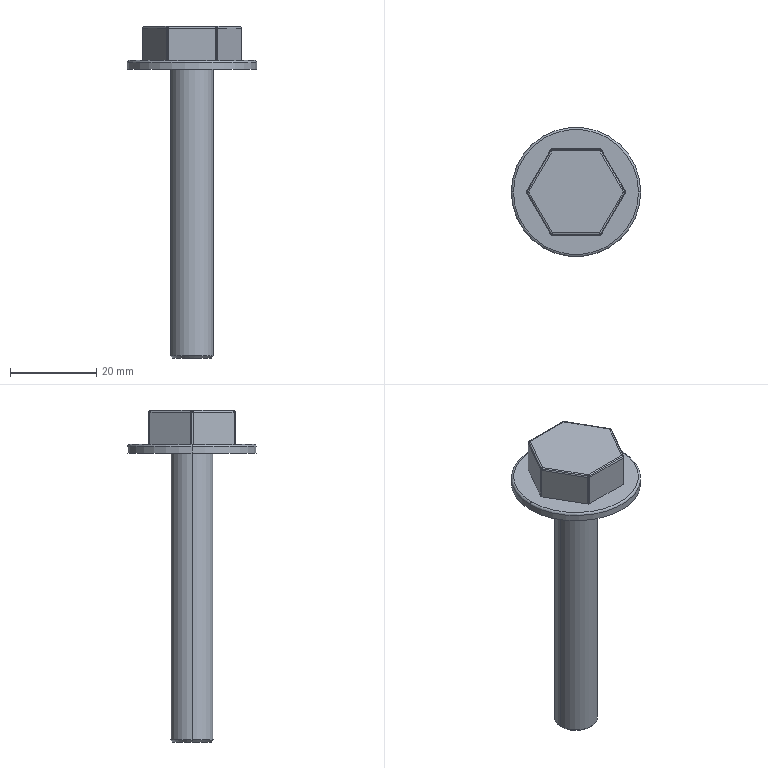Part | SolidWorks | features BaseBody 1 | 1 solid | 54 faces | box 30 x 30 x 77 mm | volume 9434 mm3 | cylinder 28 | sphere 12 | plane 10 | cone 2 | torus 2 | commonest cylinder face diameters 1 x24 10 x2 30 x2
STEP:
#1=CARTESIAN_POINT('',(4.5,0.,-67.));
#2=VERTEX_POINT('',#1);
#3=CARTESIAN_POINT('',(-4.5,0.,-67.));
#4=VERTEX_POINT('',#3);
#5=CARTESIAN_POINT('',(0.,0.,-67.));
#6=DIRECTION('',(0.,0.,1.));
#7=DIRECTION('',(1.,0.,0.));
#8=AXIS2_PLACEMENT_3D('',#5,#6,#7);
#9=CIRCLE('',#8,4.5);
#10=EDGE_CURVE('',#2,#4,#9,.T.);
#11=ORIENTED_EDGE('',*,*,#10,.T.);
#12=CARTESIAN_POINT('',(-5.,0.,-66.5));
#13=VERTEX_POINT('',#12);
#14=CARTESIAN_POINT('',(-4.75,0.,-66.75));
#15=DIRECTION('',(-0.7071,0.,0.7071));
#16=VECTOR('',#15,1000.);
#17=LINE('',#14,#16);
#18=EDGE_CURVE('',#4,#13,#17,.T.);
#19=ORIENTED_EDGE('',*,*,#18,.T.);
#20=CARTESIAN_POINT('',(5.,0.,-66.5));
#21=VERTEX_POINT('',#20);
#22=CARTESIAN_POINT('',(0.,0.,-66.5));
#23=DIRECTION('',(0.,0.,-1.));
#24=DIRECTION('',(1.,0.,0.));
#25=AXIS2_PLACEMENT_3D('',#22,#23,#24);
#26=CIRCLE('',#25,5.);
#27=EDGE_CURVE('',#13,#21,#26,.T.);
#28=ORIENTED_EDGE('',*,*,#27,.T.);
#29=CARTESIAN_POINT('',(4.75,0.,-66.75));
#30=DIRECTION('',(0.7071,0.,0.7071));
#31=VECTOR('',#30,1000.);
#32=LINE('',#29,#31);
#33=EDGE_CURVE('',#2,#21,#32,.T.);
#34=ORIENTED_EDGE('',*,*,#33,.F.);
#35=EDGE_LOOP('',(#11,#19,#28,#34));
#36=FACE_OUTER_BOUND('',#35,.T.);
#37=CARTESIAN_POINT('',(0.,0.,-66.75));
#38=DIRECTION('',(0.,0.,1.));
#39=DIRECTION('',(1.,0.,0.));
#40=AXIS2_PLACEMENT_3D('',#37,#38,#39);
#41=CONICAL_SURFACE('',#40,4.75,0.7854);
#42=ADVANCED_FACE('',(#36),#41,.T.);
#43=ORIENTED_EDGE('',*,*,#27,.F.);
#44=CARTESIAN_POINT('',(-5.,0.,0.));
#45=VERTEX_POINT('',#44);
#46=CARTESIAN_POINT('',(-5.,0.,0.));
#47=DIRECTION('',(0.,0.,1.));
#48=VECTOR('',#47,1000.);
#49=LINE('',#46,#48);
#50=EDGE_CURVE('',#13,#45,#49,.T.);
#51=ORIENTED_EDGE('',*,*,#50,.T.);
#52=CARTESIAN_POINT('',(5.,0.,0.));
#53=VERTEX_POINT('',#52);
#54=CARTESIAN_POINT('',(0.,0.,0.));
#55=DIRECTION('',(0.,0.,1.));
#56=DIRECTION('',(1.,0.,0.));
#57=AXIS2_PLACEMENT_3D('',#54,#55,#56);
#58=CIRCLE('',#57,5.);
#59=EDGE_CURVE('',#53,#45,#58,.T.);
#60=ORIENTED_EDGE('',*,*,#59,.F.);
#61=CARTESIAN_POINT('',(5.,0.,0.));
#62=DIRECTION('',(0.,0.,1.));
#63=VECTOR('',#62,1000.);
#64=LINE('',#61,#63);
#65=EDGE_CURVE('',#21,#53,#64,.T.);
#66=ORIENTED_EDGE('',*,*,#65,.F.);
#67=EDGE_LOOP('',(#43,#51,#60,#66));
#68=FACE_OUTER_BOUND('',#67,.T.);
#69=CARTESIAN_POINT('',(0.,0.,0.));
#70=DIRECTION('',(0.,0.,1.));
#71=DIRECTION('',(1.,0.,0.));
#72=AXIS2_PLACEMENT_3D('',#69,#70,#71);
#73=CYLINDRICAL_SURFACE('',#72,5.);
#74=ADVANCED_FACE('',(#68),#73,.T.);
#75=CARTESIAN_POINT('',(15.,0.,1.5));
#76=VERTEX_POINT('',#75);
#77=CARTESIAN_POINT('',(-15.,0.,1.5));
#78=VERTEX_POINT('',#77);
#79=CARTESIAN_POINT('',(0.,0.,1.5));
#80=DIRECTION('',(0.,0.,1.));
#81=DIRECTION('',(-1.,0.,0.));
#82=AXIS2_PLACEMENT_3D('',#79,#80,#81);
#83=CIRCLE('',#82,15.);
#84=EDGE_CURVE('',#76,#78,#83,.T.);
#85=ORIENTED_EDGE('',*,*,#84,.T.);
#86=CARTESIAN_POINT('',(-14.5,0.,2.));
#87=VERTEX_POINT('',#86);
#88=CARTESIAN_POINT('',(-14.5,0.,1.5));
#89=DIRECTION('',(0.,1.,0.));
#90=DIRECTION('',(-1.,0.,0.));
#91=AXIS2_PLACEMENT_3D('',#88,#89,#90);
#92=CIRCLE('',#91,0.5);
#93=EDGE_CURVE('',#78,#87,#92,.T.);
#94=ORIENTED_EDGE('',*,*,#93,.T.);
#95=CARTESIAN_POINT('',(14.5,0.,2.));
#96=VERTEX_POINT('',#95);
#97=CARTESIAN_POINT('',(0.,0.,2.));
#98=DIRECTION('',(0.,0.,-1.));
#99=DIRECTION('',(-1.,0.,0.));
#100=AXIS2_PLACEMENT_3D('',#97,#98,#99);
#101=CIRCLE('',#100,14.5);
#102=EDGE_CURVE('',#87,#96,#101,.T.);
#103=ORIENTED_EDGE('',*,*,#102,.T.);
#104=CARTESIAN_POINT('',(14.5,0.,1.5));
#105=DIRECTION('',(0.,-1.,0.));
#106=DIRECTION('',(0.,0.,-1.));
#107=AXIS2_PLACEMENT_3D('',#104,#105,#106);
#108=CIRCLE('',#107,0.5);
#109=EDGE_CURVE('',#76,#96,#108,.T.);
#110=ORIENTED_EDGE('',*,*,#109,.F.);
#111=EDGE_LOOP('',(#85,#94,#103,#110));
#112=FACE_OUTER_BOUND('',#111,.T.);
#113=CARTESIAN_POINT('',(0.,0.,1.5));
#114=DIRECTION('',(0.,0.,1.));
#115=DIRECTION('',(1.,0.,0.));
#116=AXIS2_PLACEMENT_3D('',#113,#114,#115);
#117=TOROIDAL_SURFACE('',#116,14.5,0.5);
#118=ADVANCED_FACE('',(#112),#117,.T.);
#119=ORIENTED_EDGE('',*,*,#84,.F.);
#120=CARTESIAN_POINT('',(15.,0.,0.));
#121=VERTEX_POINT('',#120);
#122=CARTESIAN_POINT('',(15.,0.,0.));
#123=DIRECTION('',(0.,0.,-1.));
#124=VECTOR('',#123,1000.);
#125=LINE('',#122,#124);
#126=EDGE_CURVE('',#76,#121,#125,.T.);
#127=ORIENTED_EDGE('',*,*,#126,.T.);
#128=CARTESIAN_POINT('',(-15.,0.,0.));
#129=VERTEX_POINT('',#128);
#130=CARTESIAN_POINT('',(0.,0.,0.));
#131=DIRECTION('',(0.,0.,-1.));
#132=DIRECTION('',(-1.,0.,0.));
#133=AXIS2_PLACEMENT_3D('',#130,#131,#132);
#134=CIRCLE('',#133,15.);
#135=EDGE_CURVE('',#129,#121,#134,.T.);
#136=ORIENTED_EDGE('',*,*,#135,.F.);
#137=CARTESIAN_POINT('',(-15.,0.,0.));
#138=DIRECTION('',(0.,0.,-1.));
#139=VECTOR('',#138,1000.);
#140=LINE('',#137,#139);
#141=EDGE_CURVE('',#78,#129,#140,.T.);
#142=ORIENTED_EDGE('',*,*,#141,.F.);
#143=EDGE_LOOP('',(#119,#127,#136,#142));
#144=FACE_OUTER_BOUND('',#143,.T.);
#145=CARTESIAN_POINT('',(0.,0.,0.));
#146=DIRECTION('',(0.,0.,-1.));
#147=DIRECTION('',(-1.,0.,0.));
#148=AXIS2_PLACEMENT_3D('',#145,#146,#147);
#149=CYLINDRICAL_SURFACE('',#148,15.);
#150=ADVANCED_FACE('',(#144),#149,.T.);
#151=CARTESIAN_POINT('',(5.646,9.593,9.964));
#152=VERTEX_POINT('',#151);
#153=CARTESIAN_POINT('',(5.485,9.5,10.));
#154=VERTEX_POINT('',#153);
#155=CARTESIAN_POINT('',(5.485,9.5,9.5));
#156=DIRECTION('',(0.5,-0.866,0.));
#157=DIRECTION('',(0.866,0.5,0.));
#158=AXIS2_PLACEMENT_3D('',#155,#156,#157);
#159=CIRCLE('',#158,0.5);
#160=EDGE_CURVE('',#152,#154,#159,.T.);
#161=ORIENTED_EDGE('',*,*,#160,.F.);
#162=CARTESIAN_POINT('',(5.67,9.964,9.5));
#163=VERTEX_POINT('',#162);
#164=CARTESIAN_POINT('',(5.485,9.5,9.5));
#165=DIRECTION('',(-0.9014,0.3603,0.2402));
#166=DIRECTION('',(-0.3712,-0.9286,0.));
#167=AXIS2_PLACEMENT_3D('',#164,#165,#166);
#168=CIRCLE('',#167,0.5);
#169=EDGE_CURVE('',#152,#163,#168,.T.);
#170=ORIENTED_EDGE('',*,*,#169,.T.);
#171=CARTESIAN_POINT('',(5.485,10.,9.5));
#172=VERTEX_POINT('',#171);
#173=CARTESIAN_POINT('',(5.485,9.5,9.5));
#174=DIRECTION('',(0.,0.,-1.));
#175=DIRECTION('',(0.,1.,0.));
#176=AXIS2_PLACEMENT_3D('',#173,#174,#175);
#177=CIRCLE('',#176,0.5);
#178=EDGE_CURVE('',#172,#163,#177,.T.);
#179=ORIENTED_EDGE('',*,*,#178,.F.);
#180=CARTESIAN_POINT('',(5.485,9.854,9.854));
#181=VERTEX_POINT('',#180);
#182=CARTESIAN_POINT('',(5.485,9.5,9.5));
#183=DIRECTION('',(-1.,0.,0.));
#184=DIRECTION('',(0.,0.,1.));
#185=AXIS2_PLACEMENT_3D('',#182,#183,#184);
#186=CIRCLE('',#185,0.5);
#187=EDGE_CURVE('',#181,#172,#186,.T.);
#188=ORIENTED_EDGE('',*,*,#187,.F.);
#189=CARTESIAN_POINT('',(5.485,9.5,9.5));
#190=DIRECTION('',(-1.,0.,0.));
#191=DIRECTION('',(0.,0.,1.));
#192=AXIS2_PLACEMENT_3D('',#189,#190,#191);
#193=CIRCLE('',#192,0.5);
#194=EDGE_CURVE('',#154,#181,#193,.T.);
#195=ORIENTED_EDGE('',*,*,#194,.F.);
#196=EDGE_LOOP('',(#161,#170,#179,#188,#195));
#197=FACE_OUTER_BOUND('',#196,.T.);
#198=CARTESIAN_POINT('',(5.485,9.5,9.5));
#199=DIRECTION('',(0.9014,-0.3603,-0.2402));
#200=DIRECTION('',(0.433,0.75,0.5));
#201=AXIS2_PLACEMENT_3D('',#198,#199,#200);
#202=SPHERICAL_SURFACE('',#201,0.5);
#203=ADVANCED_FACE('',(#197),#202,.T.);
#204=ORIENTED_EDGE('',*,*,#178,.T.);
#205=CARTESIAN_POINT('',(5.735,9.933,9.5));
#206=VERTEX_POINT('',#205);
#207=CARTESIAN_POINT('',(5.485,9.5,9.5));
#208=DIRECTION('',(0.,0.,-1.));
#209=DIRECTION('',(0.,1.,0.));
#210=AXIS2_PLACEMENT_3D('',#207,#208,#209);
#211=CIRCLE('',#210,0.5);
#212=EDGE_CURVE('',#163,#206,#211,.T.);
#213=ORIENTED_EDGE('',*,*,#212,.T.);
#214=CARTESIAN_POINT('',(5.735,9.933,2.));
#215=VERTEX_POINT('',#214);
#216=CARTESIAN_POINT('',(5.735,9.933,2.));
#217=DIRECTION('',(0.,0.,-1.));
#218=VECTOR('',#217,1000.);
#219=LINE('',#216,#218);
#220=EDGE_CURVE('',#206,#215,#219,.T.);
#221=ORIENTED_EDGE('',*,*,#220,.T.);
#222=CARTESIAN_POINT('',(5.485,10.,2.));
#223=VERTEX_POINT('',#222);
#224=CARTESIAN_POINT('',(5.485,9.5,2.));
#225=DIRECTION('',(0.,0.,1.));
#226=DIRECTION('',(0.5,0.866,0.));
#227=AXIS2_PLACEMENT_3D('',#224,#225,#226);
#228=CIRCLE('',#227,0.5);
#229=EDGE_CURVE('',#215,#223,#228,.T.);
#230=ORIENTED_EDGE('',*,*,#229,.T.);
#231=CARTESIAN_POINT('',(5.485,10.,2.));
#232=DIRECTION('',(0.,0.,1.));
#233=VECTOR('',#232,1000.);
#234=LINE('',#231,#233);
#235=EDGE_CURVE('',#223,#172,#234,.T.);
#236=ORIENTED_EDGE('',*,*,#235,.T.);
#237=EDGE_LOOP('',(#204,#213,#221,#230,#236));
#238=FACE_OUTER_BOUND('',#237,.T.);
#239=CARTESIAN_POINT('',(5.485,9.5,2.));
#240=DIRECTION('',(0.,0.,-1.));
#241=DIRECTION('',(0.5,0.866,0.));
#242=AXIS2_PLACEMENT_3D('',#239,#240,#241);
#243=CYLINDRICAL_SURFACE('',#242,0.5);
#244=ADVANCED_FACE('',(#238),#243,.T.);
#245=CARTESIAN_POINT('',(11.357,0.2236,9.724));
#246=VERTEX_POINT('',#245);
#247=CARTESIAN_POINT('',(11.403,0.25,9.5));
#248=VERTEX_POINT('',#247);
#249=CARTESIAN_POINT('',(10.97,0.,9.5));
#250=DIRECTION('',(-0.5,0.866,0.));
#251=DIRECTION('',(0.,0.,1.));
#252=AXIS2_PLACEMENT_3D('',#249,#250,#251);
#253=CIRCLE('',#252,0.5);
#254=EDGE_CURVE('',#246,#248,#253,.T.);
#255=ORIENTED_EDGE('',*,*,#254,.F.);
#256=CARTESIAN_POINT('',(11.357,-0.2236,9.724));
#257=VERTEX_POINT('',#256);
#258=CARTESIAN_POINT('',(10.97,0.,9.5));
#259=DIRECTION('',(0.5,0.,-0.866));
#260=DIRECTION('',(-0.866,0.,-0.5));
#261=AXIS2_PLACEMENT_3D('',#258,#259,#260);
#262=CIRCLE('',#261,0.5);
#263=EDGE_CURVE('',#246,#257,#262,.T.);
#264=ORIENTED_EDGE('',*,*,#263,.T.);
#265=CARTESIAN_POINT('',(11.403,-0.25,9.5));
#266=VERTEX_POINT('',#265);
#267=CARTESIAN_POINT('',(10.97,0.,9.5));
#268=DIRECTION('',(-0.5,-0.866,0.));
#269=DIRECTION('',(0.866,-0.5,0.));
#270=AXIS2_PLACEMENT_3D('',#267,#268,#269);
#271=CIRCLE('',#270,0.5);
#272=EDGE_CURVE('',#266,#257,#271,.T.);
#273=ORIENTED_EDGE('',*,*,#272,.F.);
#274=CARTESIAN_POINT('',(11.47,0.,9.5));
#275=VERTEX_POINT('',#274);
#276=CARTESIAN_POINT('',(10.97,0.,9.5));
#277=DIRECTION('',(0.,0.,-1.));
#278=DIRECTION('',(0.866,0.5,0.));
#279=AXIS2_PLACEMENT_3D('',#276,#277,#278);
#280=CIRCLE('',#279,0.5);
#281=EDGE_CURVE('',#275,#266,#280,.T.);
#282=ORIENTED_EDGE('',*,*,#281,.F.);
#283=CARTESIAN_POINT('',(10.97,0.,9.5));
#284=DIRECTION('',(0.,0.,-1.));
#285=DIRECTION('',(0.866,0.5,0.));
#286=AXIS2_PLACEMENT_3D('',#283,#284,#285);
#287=CIRCLE('',#286,0.5);
#288=EDGE_CURVE('',#248,#275,#287,.T.);
#289=ORIENTED_EDGE('',*,*,#288,.F.);
#290=EDGE_LOOP('',(#255,#264,#273,#282,#289));
#291=FACE_OUTER_BOUND('',#290,.T.);
#292=CARTESIAN_POINT('',(10.97,0.,9.5));
#293=DIRECTION('',(-0.5,0.,0.866));
#294=DIRECTION('',(0.866,0.,0.5));
#295=AXIS2_PLACEMENT_3D('',#292,#293,#294);
#296=SPHERICAL_SURFACE('',#295,0.5);
#297=ADVANCED_FACE('',(#291),#296,.T.);
#298=ORIENTED_EDGE('',*,*,#288,.T.);
#299=CARTESIAN_POINT('',(11.47,0.,2.));
#300=VERTEX_POINT('',#299);
#301=CARTESIAN_POINT('',(11.47,0.,2.));
#302=DIRECTION('',(0.,0.,-1.));
#303=VECTOR('',#302,1000.);
#304=LINE('',#301,#303);
#305=EDGE_CURVE('',#275,#300,#304,.T.);
#306=ORIENTED_EDGE('',*,*,#305,.T.);
#307=CARTESIAN_POINT('',(11.403,0.25,2.));
#308=VERTEX_POINT('',#307);
#309=CARTESIAN_POINT('',(10.97,0.,2.));
#310=DIRECTION('',(0.,0.,1.));
#311=DIRECTION('',(1.,0.,0.));
#312=AXIS2_PLACEMENT_3D('',#309,#310,#311);
#313=CIRCLE('',#312,0.5);
#314=EDGE_CURVE('',#300,#308,#313,.T.);
#315=ORIENTED_EDGE('',*,*,#314,.T.);
#316=CARTESIAN_POINT('',(11.403,0.25,2.));
#317=DIRECTION('',(0.,0.,1.));
#318=VECTOR('',#317,1000.);
#319=LINE('',#316,#318);
#320=EDGE_CURVE('',#308,#248,#319,.T.);
#321=ORIENTED_EDGE('',*,*,#320,.T.);
#322=EDGE_LOOP('',(#298,#306,#315,#321));
#323=FACE_OUTER_BOUND('',#322,.T.);
#324=CARTESIAN_POINT('',(10.97,0.,2.));
#325=DIRECTION('',(0.,0.,-1.));
#326=DIRECTION('',(1.,0.,0.));
#327=AXIS2_PLACEMENT_3D('',#324,#325,#326);
#328=CYLINDRICAL_SURFACE('',#327,0.5);
#329=ADVANCED_FACE('',(#323),#328,.T.);
#330=CARTESIAN_POINT('',(5.918,9.75,9.5));
#331=VERTEX_POINT('',#330);
#332=CARTESIAN_POINT('',(5.791,9.677,9.854));
#333=VERTEX_POINT('',#332);
#334=CARTESIAN_POINT('',(5.485,9.5,9.5));
#335=DIRECTION('',(0.5,-0.866,0.));
#336=DIRECTION('',(0.866,0.5,0.));
#337=AXIS2_PLACEMENT_3D('',#334,#335,#336);
#338=CIRCLE('',#337,0.5);
#339=EDGE_CURVE('',#331,#333,#338,.T.);
#340=ORIENTED_EDGE('',*,*,#339,.T.);
#341=CARTESIAN_POINT('',(11.276,0.1768,9.854));
#342=VERTEX_POINT('',#341);
#343=CARTESIAN_POINT('',(9.977,2.427,9.854));
#344=DIRECTION('',(0.5,-0.866,0.));
#345=VECTOR('',#344,1000.);
#346=LINE('',#343,#345);
#347=EDGE_CURVE('',#333,#342,#346,.T.);
#348=ORIENTED_EDGE('',*,*,#347,.T.);
#349=CARTESIAN_POINT('',(10.97,0.,9.5));
#350=DIRECTION('',(-0.5,0.866,0.));
#351=DIRECTION('',(0.,0.,1.));
#352=AXIS2_PLACEMENT_3D('',#349,#350,#351);
#353=CIRCLE('',#352,0.5);
#354=EDGE_CURVE('',#342,#246,#353,.T.);
#355=ORIENTED_EDGE('',*,*,#354,.T.);
#356=ORIENTED_EDGE('',*,*,#254,.T.);
#357=CARTESIAN_POINT('',(10.104,2.5,9.5));
#358=DIRECTION('',(-0.5,0.866,0.));
#359=VECTOR('',#358,1000.);
#360=LINE('',#357,#359);
#361=EDGE_CURVE('',#248,#331,#360,.T.);
#362=ORIENTED_EDGE('',*,*,#361,.T.);
#363=EDGE_LOOP('',(#340,#348,#355,#356,#362));
#364=FACE_OUTER_BOUND('',#363,.T.);
#365=CARTESIAN_POINT('',(9.671,2.25,9.5));
#366=DIRECTION('',(0.5,-0.866,0.));
#367=DIRECTION('',(0.6124,0.3536,0.7071));
#368=AXIS2_PLACEMENT_3D('',#365,#366,#367);
#369=CYLINDRICAL_SURFACE('',#368,0.5);
#370=ADVANCED_FACE('',(#364),#369,.T.);
#371=CARTESIAN_POINT('',(-5.646,9.593,9.964));
#372=VERTEX_POINT('',#371);
#373=CARTESIAN_POINT('',(-5.791,9.677,9.854));
#374=VERTEX_POINT('',#373);
#375=CARTESIAN_POINT('',(-5.485,9.5,9.5));
#376=DIRECTION('',(-0.5,-0.866,0.));
#377=DIRECTION('',(0.,0.,1.));
#378=AXIS2_PLACEMENT_3D('',#375,#376,#377);
#379=CIRCLE('',#378,0.5);
#380=EDGE_CURVE('',#372,#374,#379,.T.);
#381=ORIENTED_EDGE('',*,*,#380,.F.);
#382=CARTESIAN_POINT('',(-5.67,9.964,9.5));
#383=VERTEX_POINT('',#382);
#384=CARTESIAN_POINT('',(-5.485,9.5,9.5));
#385=DIRECTION('',(-0.9014,-0.3603,-0.2402));
#386=DIRECTION('',(0.3712,-0.9286,0.));
#387=AXIS2_PLACEMENT_3D('',#384,#385,#386);
#388=CIRCLE('',#387,0.5);
#389=EDGE_CURVE('',#372,#383,#388,.T.);
#390=ORIENTED_EDGE('',*,*,#389,.T.);
#391=CARTESIAN_POINT('',(-5.735,9.933,9.5));
#392=VERTEX_POINT('',#391);
#393=CARTESIAN_POINT('',(-5.485,9.5,9.5));
#394=DIRECTION('',(0.,0.,-1.));
#395=DIRECTION('',(-0.866,0.5,0.));
#396=AXIS2_PLACEMENT_3D('',#393,#394,#395);
#397=CIRCLE('',#396,0.5);
#398=EDGE_CURVE('',#392,#383,#397,.T.);
#399=ORIENTED_EDGE('',*,*,#398,.F.);
#400=CARTESIAN_POINT('',(-5.918,9.75,9.5));
#401=VERTEX_POINT('',#400);
#402=CARTESIAN_POINT('',(-5.485,9.5,9.5));
#403=DIRECTION('',(0.,0.,-1.));
#404=DIRECTION('',(-0.866,0.5,0.));
#405=AXIS2_PLACEMENT_3D('',#402,#403,#404);
#406=CIRCLE('',#405,0.5);
#407=EDGE_CURVE('',#401,#392,#406,.T.);
#408=ORIENTED_EDGE('',*,*,#407,.F.);
#409=CARTESIAN_POINT('',(-5.485,9.5,9.5));
#410=DIRECTION('',(-0.5,-0.866,0.));
#411=DIRECTION('',(0.,0.,1.));
#412=AXIS2_PLACEMENT_3D('',#409,#410,#411);
#413=CIRCLE('',#412,0.5);
#414=EDGE_CURVE('',#374,#401,#413,.T.);
#415=ORIENTED_EDGE('',*,*,#414,.F.);
#416=EDGE_LOOP('',(#381,#390,#399,#408,#415));
#417=FACE_OUTER_BOUND('',#416,.T.);
#418=CARTESIAN_POINT('',(-5.485,9.5,9.5));
#419=DIRECTION('',(0.9014,0.3603,0.2402));
#420=DIRECTION('',(-0.433,0.75,0.5));
#421=AXIS2_PLACEMENT_3D('',#418,#419,#420);
#422=SPHERICAL_SURFACE('',#421,0.5);
#423=ADVANCED_FACE('',(#417),#422,.T.);
#424=ORIENTED_EDGE('',*,*,#407,.T.);
#425=CARTESIAN_POINT('',(-5.735,9.933,2.));
#426=VERTEX_POINT('',#425);
#427=CARTESIAN_POINT('',(-5.735,9.933,2.));
#428=DIRECTION('',(0.,0.,-1.));
#429=VECTOR('',#428,1000.);
#430=LINE('',#427,#429);
#431=EDGE_CURVE('',#392,#426,#430,.T.);
#432=ORIENTED_EDGE('',*,*,#431,.T.);
#433=CARTESIAN_POINT('',(-5.918,9.75,2.));
#434=VERTEX_POINT('',#433);
#435=CARTESIAN_POINT('',(-5.485,9.5,2.));
#436=DIRECTION('',(0.,0.,1.));
#437=DIRECTION('',(-0.5,0.866,0.));
#438=AXIS2_PLACEMENT_3D('',#435,#436,#437);
#439=CIRCLE('',#438,0.5);
#440=EDGE_CURVE('',#426,#434,#439,.T.);
#441=ORIENTED_EDGE('',*,*,#440,.T.);
#442=CARTESIAN_POINT('',(-5.918,9.75,2.));
#443=DIRECTION('',(0.,0.,1.));
#444=VECTOR('',#443,1000.);
#445=LINE('',#442,#444);
#446=EDGE_CURVE('',#434,#401,#445,.T.);
#447=ORIENTED_EDGE('',*,*,#446,.T.);
#448=EDGE_LOOP('',(#424,#432,#441,#447));
#449=FACE_OUTER_BOUND('',#448,.T.);
#450=CARTESIAN_POINT('',(-5.485,9.5,2.));
#451=DIRECTION('',(0.,0.,-1.));
#452=DIRECTION('',(-0.5,0.866,0.));
#453=AXIS2_PLACEMENT_3D('',#450,#451,#452);
#454=CYLINDRICAL_SURFACE('',#453,0.5);
#455=ADVANCED_FACE('',(#449),#454,.T.);
#456=CARTESIAN_POINT('',(5.67,-9.964,9.5));
#457=VERTEX_POINT('',#456);
#458=CARTESIAN_POINT('',(5.485,-10.,9.5));
#459=VERTEX_POINT('',#458);
#460=CARTESIAN_POINT('',(5.485,-9.5,9.5));
#461=DIRECTION('',(0.,0.,-1.));
#462=DIRECTION('',(0.866,-0.5,0.));
#463=AXIS2_PLACEMENT_3D('',#460,#461,#462);
#464=CIRCLE('',#463,0.5);
#465=EDGE_CURVE('',#457,#459,#464,.T.);
#466=ORIENTED_EDGE('',*,*,#465,.F.);
#467=CARTESIAN_POINT('',(5.646,-9.593,9.964));
#468=VERTEX_POINT('',#467);
#469=CARTESIAN_POINT('',(5.485,-9.5,9.5));
#470=DIRECTION('',(-0.9014,-0.3603,0.2402));
#471=DIRECTION('',(0.3712,-0.9286,0.));
#472=AXIS2_PLACEMENT_3D('',#469,#470,#471);
#473=CIRCLE('',#472,0.5);
#474=EDGE_CURVE('',#457,#468,#473,.T.);
#475=ORIENTED_EDGE('',*,*,#474,.T.);
#476=CARTESIAN_POINT('',(5.485,-9.5,10.));
#477=VERTEX_POINT('',#476);
#478=CARTESIAN_POINT('',(5.485,-9.5,9.5));
#479=DIRECTION('',(0.5,0.866,0.));
#480=DIRECTION('',(0.,0.,1.));
#481=AXIS2_PLACEMENT_3D('',#478,#479,#480);
#482=CIRCLE('',#481,0.5);
#483=EDGE_CURVE('',#477,#468,#482,.T.);
#484=ORIENTED_EDGE('',*,*,#483,.F.);
#485=CARTESIAN_POINT('',(5.485,-9.854,9.854));
#486=VERTEX_POINT('',#485);
#487=CARTESIAN_POINT('',(5.485,-9.5,9.5));
#488=DIRECTION('',(-1.,0.,0.));
#489=DIRECTION('',(0.,-1.,0.));
#490=AXIS2_PLACEMENT_3D('',#487,#488,#489);
#491=CIRCLE('',#490,0.5);
#492=EDGE_CURVE('',#486,#477,#491,.T.);
#493=ORIENTED_EDGE('',*,*,#492,.F.);
#494=CARTESIAN_POINT('',(5.485,-9.5,9.5));
#495=DIRECTION('',(-1.,0.,0.));
#496=DIRECTION('',(0.,-1.,0.));
#497=AXIS2_PLACEMENT_3D('',#494,#495,#496);
#498=CIRCLE('',#497,0.5);
#499=EDGE_CURVE('',#459,#486,#498,.T.);
#500=ORIENTED_EDGE('',*,*,#499,.F.);
#501=EDGE_LOOP('',(#466,#475,#484,#493,#500));
#502=FACE_OUTER_BOUND('',#501,.T.);
#503=CARTESIAN_POINT('',(5.485,-9.5,9.5));
#504=DIRECTION('',(0.9014,0.3603,-0.2402));
#505=DIRECTION('',(0.433,-0.75,0.5));
#506=AXIS2_PLACEMENT_3D('',#503,#504,#505);
#507=SPHERICAL_SURFACE('',#506,0.5);
#508=ADVANCED_FACE('',(#502),#507,.T.);
#509=CARTESIAN_POINT('',(5.918,-9.75,9.5));
#510=VERTEX_POINT('',#509);
#511=CARTESIAN_POINT('',(5.735,-9.933,9.5));
#512=VERTEX_POINT('',#511);
#513=CARTESIAN_POINT('',(5.485,-9.5,9.5));
#514=DIRECTION('',(0.,0.,-1.));
#515=DIRECTION('',(0.866,-0.5,0.));
#516=AXIS2_PLACEMENT_3D('',#513,#514,#515);
#517=CIRCLE('',#516,0.5);
#518=EDGE_CURVE('',#510,#512,#517,.T.);
#519=ORIENTED_EDGE('',*,*,#518,.T.);
#520=CARTESIAN_POINT('',(5.735,-9.933,2.));
#521=VERTEX_POINT('',#520);
#522=CARTESIAN_POINT('',(5.735,-9.933,2.));
#523=DIRECTION('',(0.,0.,-1.));
#524=VECTOR('',#523,1000.);
#525=LINE('',#522,#524);
#526=EDGE_CURVE('',#512,#521,#525,.T.);
#527=ORIENTED_EDGE('',*,*,#526,.T.);
#528=CARTESIAN_POINT('',(5.918,-9.75,2.));
#529=VERTEX_POINT('',#528);
#530=CARTESIAN_POINT('',(5.485,-9.5,2.));
#531=DIRECTION('',(0.,0.,1.));
#532=DIRECTION('',(0.5,-0.866,0.));
#533=AXIS2_PLACEMENT_3D('',#530,#531,#532);
#534=CIRCLE('',#533,0.5);
#535=EDGE_CURVE('',#521,#529,#534,.T.);
#536=ORIENTED_EDGE('',*,*,#535,.T.);
#537=CARTESIAN_POINT('',(5.918,-9.75,2.));
#538=DIRECTION('',(0.,0.,1.));
#539=VECTOR('',#538,1000.);
#540=LINE('',#537,#539);
#541=EDGE_CURVE('',#529,#510,#540,.T.);
#542=ORIENTED_EDGE('',*,*,#541,.T.);
#543=EDGE_LOOP('',(#519,#527,#536,#542));
#544=FACE_OUTER_BOUND('',#543,.T.);
#545=CARTESIAN_POINT('',(5.485,-9.5,2.));
#546=DIRECTION('',(0.,0.,-1.));
#547=DIRECTION('',(0.5,-0.866,0.));
#548=AXIS2_PLACEMENT_3D('',#545,#546,#547);
#549=CYLINDRICAL_SURFACE('',#548,0.5);
#550=ADVANCED_FACE('',(#544),#549,.T.);
#551=ORIENTED_EDGE('',*,*,#272,.T.);
#552=CARTESIAN_POINT('',(11.276,-0.1768,9.854));
#553=VERTEX_POINT('',#552);
#554=CARTESIAN_POINT('',(10.97,0.,9.5));
#555=DIRECTION('',(-0.5,-0.866,0.));
#556=DIRECTION('',(0.866,-0.5,0.));
#557=AXIS2_PLACEMENT_3D('',#554,#555,#556);
#558=CIRCLE('',#557,0.5);
#559=EDGE_CURVE('',#257,#553,#558,.T.);
#560=ORIENTED_EDGE('',*,*,#559,.T.);
#561=CARTESIAN_POINT('',(5.791,-9.677,9.854));
#562=VERTEX_POINT('',#561);
#563=CARTESIAN_POINT('',(7.09,-7.427,9.854));
#564=DIRECTION('',(-0.5,-0.866,0.));
#565=VECTOR('',#564,1000.);
#566=LINE('',#563,#565);
#567=EDGE_CURVE('',#553,#562,#566,.T.);
#568=ORIENTED_EDGE('',*,*,#567,.T.);
#569=CARTESIAN_POINT('',(5.485,-9.5,9.5));
#570=DIRECTION('',(0.5,0.866,0.));
#571=DIRECTION('',(0.,0.,1.));
#572=AXIS2_PLACEMENT_3D('',#569,#570,#571);
#573=CIRCLE('',#572,0.5);
#574=EDGE_CURVE('',#562,#510,#573,.T.);
#575=ORIENTED_EDGE('',*,*,#574,.T.);
#576=CARTESIAN_POINT('',(7.217,-7.5,9.5));
#577=DIRECTION('',(0.5,0.866,0.));
#578=VECTOR('',#577,1000.);
#579=LINE('',#576,#578);
#580=EDGE_CURVE('',#510,#266,#579,.T.);
#581=ORIENTED_EDGE('',*,*,#580,.T.);
#582=EDGE_LOOP('',(#551,#560,#568,#575,#581));
#583=FACE_OUTER_BOUND('',#582,.T.);
#584=CARTESIAN_POINT('',(6.784,-7.25,9.5));
#585=DIRECTION('',(-0.5,-0.866,0.));
#586=DIRECTION('',(0.6124,-0.3536,0.7071));
#587=AXIS2_PLACEMENT_3D('',#584,#585,#586);
#588=CYLINDRICAL_SURFACE('',#587,0.5);
#589=ADVANCED_FACE('',(#583),#588,.T.);
#590=CARTESIAN_POINT('',(-11.357,-0.2236,9.724));
#591=VERTEX_POINT('',#590);
#592=CARTESIAN_POINT('',(-11.403,-0.25,9.5));
#593=VERTEX_POINT('',#592);
#594=CARTESIAN_POINT('',(-10.97,0.,9.5));
#595=DIRECTION('',(0.5,-0.866,0.));
#596=DIRECTION('',(0.,0.,1.));
#597=AXIS2_PLACEMENT_3D('',#594,#595,#596);
#598=CIRCLE('',#597,0.5);
#599=EDGE_CURVE('',#591,#593,#598,.T.);
#600=ORIENTED_EDGE('',*,*,#599,.F.);
#601=CARTESIAN_POINT('',(-11.357,0.2236,9.724));
#602=VERTEX_POINT('',#601);
#603=CARTESIAN_POINT('',(-10.97,0.,9.5));
#604=DIRECTION('',(-0.5,0.,-0.866));
#605=DIRECTION('',(-0.866,0.,0.5));
#606=AXIS2_PLACEMENT_3D('',#603,#604,#605);
#607=CIRCLE('',#606,0.5);
#608=EDGE_CURVE('',#591,#602,#607,.T.);
#609=ORIENTED_EDGE('',*,*,#608,.T.);
#610=CARTESIAN_POINT('',(-11.403,0.25,9.5));
#611=VERTEX_POINT('',#610);
#612=CARTESIAN_POINT('',(-10.97,0.,9.5));
#613=DIRECTION('',(0.5,0.866,0.));
#614=DIRECTION('',(-0.866,0.5,0.));
#615=AXIS2_PLACEMENT_3D('',#612,#613,#614);
#616=CIRCLE('',#615,0.5);
#617=EDGE_CURVE('',#611,#602,#616,.T.);
#618=ORIENTED_EDGE('',*,*,#617,.F.);
#619=CARTESIAN_POINT('',(-11.47,0.,9.5));
#620=VERTEX_POINT('',#619);
#621=CARTESIAN_POINT('',(-10.97,0.,9.5));
#622=DIRECTION('',(0.,0.,-1.));
#623=DIRECTION('',(-0.866,-0.5,0.));
#624=AXIS2_PLACEMENT_3D('',#621,#622,#623);
#625=CIRCLE('',#624,0.5);
#626=EDGE_CURVE('',#620,#611,#625,.T.);
#627=ORIENTED_EDGE('',*,*,#626,.F.);
#628=CARTESIAN_POINT('',(-10.97,0.,9.5));
#629=DIRECTION('',(0.,0.,-1.));
#630=DIRECTION('',(-0.866,-0.5,0.));
#631=AXIS2_PLACEMENT_3D('',#628,#629,#630);
#632=CIRCLE('',#631,0.5);
#633=EDGE_CURVE('',#593,#620,#632,.T.);
#634=ORIENTED_EDGE('',*,*,#633,.F.);
#635=EDGE_LOOP('',(#600,#609,#618,#627,#634));
#636=FACE_OUTER_BOUND('',#635,.T.);
#637=CARTESIAN_POINT('',(-10.97,0.,9.5));
#638=DIRECTION('',(0.5,0.,0.866));
#639=DIRECTION('',(-0.866,0.,0.5));
#640=AXIS2_PLACEMENT_3D('',#637,#638,#639);
#641=SPHERICAL_SURFACE('',#640,0.5);
#642=ADVANCED_FACE('',(#636),#641,.T.);
#643=ORIENTED_EDGE('',*,*,#633,.T.);
#644=CARTESIAN_POINT('',(-11.47,0.,2.));
#645=VERTEX_POINT('',#644);
#646=CARTESIAN_POINT('',(-11.47,0.,2.));
#647=DIRECTION('',(0.,0.,-1.));
#648=VECTOR('',#647,1000.);
#649=LINE('',#646,#648);
#650=EDGE_CURVE('',#620,#645,#649,.T.);
#651=ORIENTED_EDGE('',*,*,#650,.T.);
#652=CARTESIAN_POINT('',(-11.403,-0.25,2.));
#653=VERTEX_POINT('',#652);
#654=CARTESIAN_POINT('',(-10.97,0.,2.));
#655=DIRECTION('',(0.,0.,1.));
#656=DIRECTION('',(-1.,0.,0.));
#657=AXIS2_PLACEMENT_3D('',#654,#655,#656);
#658=CIRCLE('',#657,0.5);
#659=EDGE_CURVE('',#645,#653,#658,.T.);
#660=ORIENTED_EDGE('',*,*,#659,.T.);
#661=CARTESIAN_POINT('',(-11.403,-0.25,2.));
#662=DIRECTION('',(0.,0.,1.));
#663=VECTOR('',#662,1000.);
#664=LINE('',#661,#663);
#665=EDGE_CURVE('',#653,#593,#664,.T.);
#666=ORIENTED_EDGE('',*,*,#665,.T.);
#667=EDGE_LOOP('',(#643,#651,#660,#666));
#668=FACE_OUTER_BOUND('',#667,.T.);
#669=CARTESIAN_POINT('',(-10.97,0.,2.));
#670=DIRECTION('',(0.,0.,-1.));
#671=DIRECTION('',(-1.,0.,0.));
#672=AXIS2_PLACEMENT_3D('',#669,#670,#671);
#673=CYLINDRICAL_SURFACE('',#672,0.5);
#674=ADVANCED_FACE('',(#668),#673,.T.);
#675=CARTESIAN_POINT('',(-5.67,-9.964,9.5));
#676=VERTEX_POINT('',#675);
#677=CARTESIAN_POINT('',(-5.735,-9.933,9.5));
#678=VERTEX_POINT('',#677);
#679=CARTESIAN_POINT('',(-5.485,-9.5,9.5));
#680=DIRECTION('',(0.,0.,-1.));
#681=DIRECTION('',(0.,-1.,0.));
#682=AXIS2_PLACEMENT_3D('',#679,#680,#681);
#683=CIRCLE('',#682,0.5);
#684=EDGE_CURVE('',#676,#678,#683,.T.);
#685=ORIENTED_EDGE('',*,*,#684,.F.);
#686=CARTESIAN_POINT('',(-5.646,-9.593,9.964));
#687=VERTEX_POINT('',#686);
#688=CARTESIAN_POINT('',(-5.485,-9.5,9.5));
#689=DIRECTION('',(-0.9014,0.3603,-0.2402));
#690=DIRECTION('',(-0.3712,-0.9286,0.));
#691=AXIS2_PLACEMENT_3D('',#688,#689,#690);
#692=CIRCLE('',#691,0.5);
#693=EDGE_CURVE('',#676,#687,#692,.T.);
#694=ORIENTED_EDGE('',*,*,#693,.T.);
#695=CARTESIAN_POINT('',(-5.791,-9.677,9.854));
#696=VERTEX_POINT('',#695);
#697=CARTESIAN_POINT('',(-5.485,-9.5,9.5));
#698=DIRECTION('',(-0.5,0.866,0.));
#699=DIRECTION('',(-0.866,-0.5,0.));
#700=AXIS2_PLACEMENT_3D('',#697,#698,#699);
#701=CIRCLE('',#700,0.5);
#702=EDGE_CURVE('',#696,#687,#701,.T.);
#703=ORIENTED_EDGE('',*,*,#702,.F.);
#704=CARTESIAN_POINT('',(-5.918,-9.75,9.5));
#705=VERTEX_POINT('',#704);
#706=CARTESIAN_POINT('',(-5.485,-9.5,9.5));
#707=DIRECTION('',(-0.5,0.866,0.));
#708=DIRECTION('',(-0.866,-0.5,0.));
#709=AXIS2_PLACEMENT_3D('',#706,#707,#708);
#710=CIRCLE('',#709,0.5);
#711=EDGE_CURVE('',#705,#696,#710,.T.);
#712=ORIENTED_EDGE('',*,*,#711,.F.);
#713=CARTESIAN_POINT('',(-5.485,-9.5,9.5));
#714=DIRECTION('',(0.,0.,-1.));
#715=DIRECTION('',(0.,-1.,0.));
#716=AXIS2_PLACEMENT_3D('',#713,#714,#715);
#717=CIRCLE('',#716,0.5);
#718=EDGE_CURVE('',#678,#705,#717,.T.);
#719=ORIENTED_EDGE('',*,*,#718,.F.);
#720=EDGE_LOOP('',(#685,#694,#703,#712,#719));
#721=FACE_OUTER_BOUND('',#720,.T.);
#722=CARTESIAN_POINT('',(-5.485,-9.5,9.5));
#723=DIRECTION('',(0.9014,-0.3603,0.2402));
#724=DIRECTION('',(-0.433,-0.75,0.5));
#725=AXIS2_PLACEMENT_3D('',#722,#723,#724);
#726=SPHERICAL_SURFACE('',#725,0.5);
#727=ADVANCED_FACE('',(#721),#726,.T.);
#728=CARTESIAN_POINT('',(-5.485,-10.,9.5));
#729=VERTEX_POINT('',#728);
#730=CARTESIAN_POINT('',(-5.485,-9.5,9.5));
#731=DIRECTION('',(0.,0.,-1.));
#732=DIRECTION('',(0.,-1.,0.));
#733=AXIS2_PLACEMENT_3D('',#730,#731,#732);
#734=CIRCLE('',#733,0.5);
#735=EDGE_CURVE('',#729,#676,#734,.T.);
#736=ORIENTED_EDGE('',*,*,#735,.T.);
#737=ORIENTED_EDGE('',*,*,#684,.T.);
#738=CARTESIAN_POINT('',(-5.735,-9.933,2.));
#739=VERTEX_POINT('',#738);
#740=CARTESIAN_POINT('',(-5.735,-9.933,2.));
#741=DIRECTION('',(0.,0.,-1.));
#742=VECTOR('',#741,1000.);
#743=LINE('',#740,#742);
#744=EDGE_CURVE('',#678,#739,#743,.T.);
#745=ORIENTED_EDGE('',*,*,#744,.T.);
#746=CARTESIAN_POINT('',(-5.485,-10.,2.));
#747=VERTEX_POINT('',#746);
#748=CARTESIAN_POINT('',(-5.485,-9.5,2.));
#749=DIRECTION('',(0.,0.,1.));
#750=DIRECTION('',(-0.5,-0.866,0.));
#751=AXIS2_PLACEMENT_3D('',#748,#749,#750);
#752=CIRCLE('',#751,0.5);
#753=EDGE_CURVE('',#739,#747,#752,.T.);
#754=ORIENTED_EDGE('',*,*,#753,.T.);
#755=CARTESIAN_POINT('',(-5.485,-10.,2.));
#756=DIRECTION('',(0.,0.,1.));
#757=VECTOR('',#756,1000.);
#758=LINE('',#755,#757);
#759=EDGE_CURVE('',#747,#729,#758,.T.);
#760=ORIENTED_EDGE('',*,*,#759,.T.);
#761=EDGE_LOOP('',(#736,#737,#745,#754,#760));
#762=FACE_OUTER_BOUND('',#761,.T.);
#763=CARTESIAN_POINT('',(-5.485,-9.5,2.));
#764=DIRECTION('',(0.,0.,-1.));
#765=DIRECTION('',(-0.5,-0.866,0.));
#766=AXIS2_PLACEMENT_3D('',#763,#764,#765);
#767=CYLINDRICAL_SURFACE('',#766,0.5);
#768=ADVANCED_FACE('',(#762),#767,.T.);
#769=ORIENTED_EDGE('',*,*,#499,.T.);
#770=CARTESIAN_POINT('',(-5.485,-9.854,9.854));
#771=VERTEX_POINT('',#770);
#772=CARTESIAN_POINT('',(-2.887,-9.854,9.854));
#773=DIRECTION('',(-1.,0.,0.));
#774=VECTOR('',#773,1000.);
#775=LINE('',#772,#774);
#776=EDGE_CURVE('',#486,#771,#775,.T.);
#777=ORIENTED_EDGE('',*,*,#776,.T.);
#778=CARTESIAN_POINT('',(-5.485,-9.5,9.5));
#779=DIRECTION('',(1.,0.,0.));
#780=DIRECTION('',(0.,0.,1.));
#781=AXIS2_PLACEMENT_3D('',#778,#779,#780);
#782=CIRCLE('',#781,0.5);
#783=EDGE_CURVE('',#771,#729,#782,.T.);
#784=ORIENTED_EDGE('',*,*,#783,.T.);
#785=CARTESIAN_POINT('',(-2.887,-10.,9.5));
#786=DIRECTION('',(1.,0.,0.));
#787=VECTOR('',#786,1000.);
#788=LINE('',#785,#787);
#789=EDGE_CURVE('',#729,#459,#788,.T.);
#790=ORIENTED_EDGE('',*,*,#789,.T.);
#791=EDGE_LOOP('',(#769,#777,#784,#790));
#792=FACE_OUTER_BOUND('',#791,.T.);
#793=CARTESIAN_POINT('',(-2.887,-9.5,9.5));
#794=DIRECTION('',(-1.,0.,0.));
#795=DIRECTION('',(0.,-0.7071,0.7071));
#796=AXIS2_PLACEMENT_3D('',#793,#794,#795);
#797=CYLINDRICAL_SURFACE('',#796,0.5);
#798=ADVANCED_FACE('',(#792),#797,.T.);
#799=ORIENTED_EDGE('',*,*,#711,.T.);
#800=CARTESIAN_POINT('',(-11.276,-0.1768,9.854));
#801=VERTEX_POINT('',#800);
#802=CARTESIAN_POINT('',(-9.977,-2.427,9.854));
#803=DIRECTION('',(-0.5,0.866,0.));
#804=VECTOR('',#803,1000.);
#805=LINE('',#802,#804);
#806=EDGE_CURVE('',#696,#801,#805,.T.);
#807=ORIENTED_EDGE('',*,*,#806,.T.);
#808=CARTESIAN_POINT('',(-10.97,0.,9.5));
#809=DIRECTION('',(0.5,-0.866,0.));
#810=DIRECTION('',(0.,0.,1.));
#811=AXIS2_PLACEMENT_3D('',#808,#809,#810);
#812=CIRCLE('',#811,0.5);
#813=EDGE_CURVE('',#801,#591,#812,.T.);
#814=ORIENTED_EDGE('',*,*,#813,.T.);
#815=ORIENTED_EDGE('',*,*,#599,.T.);
#816=CARTESIAN_POINT('',(-10.104,-2.5,9.5));
#817=DIRECTION('',(0.5,-0.866,0.));
#818=VECTOR('',#817,1000.);
#819=LINE('',#816,#818);
#820=EDGE_CURVE('',#593,#705,#819,.T.);
#821=ORIENTED_EDGE('',*,*,#820,.T.);
#822=EDGE_LOOP('',(#799,#807,#814,#815,#821));
#823=FACE_OUTER_BOUND('',#822,.T.);
#824=CARTESIAN_POINT('',(-9.671,-2.25,9.5));
#825=DIRECTION('',(-0.5,0.866,0.));
#826=DIRECTION('',(-0.6124,-0.3536,0.7071));
#827=AXIS2_PLACEMENT_3D('',#824,#825,#826);
#828=CYLINDRICAL_SURFACE('',#827,0.5);
#829=ADVANCED_FACE('',(#823),#828,.T.);
#830=ORIENTED_EDGE('',*,*,#617,.T.);
#831=CARTESIAN_POINT('',(-11.276,0.1768,9.854));
#832=VERTEX_POINT('',#831);
#833=CARTESIAN_POINT('',(-10.97,0.,9.5));
#834=DIRECTION('',(0.5,0.866,0.));
#835=DIRECTION('',(-0.866,0.5,0.));
#836=AXIS2_PLACEMENT_3D('',#833,#834,#835);
#837=CIRCLE('',#836,0.5);
#838=EDGE_CURVE('',#602,#832,#837,.T.);
#839=ORIENTED_EDGE('',*,*,#838,.T.);
#840=CARTESIAN_POINT('',(-7.09,7.427,9.854));
#841=DIRECTION('',(0.5,0.866,0.));
#842=VECTOR('',#841,1000.);
#843=LINE('',#840,#842);
#844=EDGE_CURVE('',#832,#374,#843,.T.);
#845=ORIENTED_EDGE('',*,*,#844,.T.);
#846=ORIENTED_EDGE('',*,*,#414,.T.);
#847=CARTESIAN_POINT('',(-7.217,7.5,9.5));
#848=DIRECTION('',(-0.5,-0.866,0.));
#849=VECTOR('',#848,1000.);
#850=LINE('',#847,#849);
#851=EDGE_CURVE('',#401,#611,#850,.T.);
#852=ORIENTED_EDGE('',*,*,#851,.T.);
#853=EDGE_LOOP('',(#830,#839,#845,#846,#852));
#854=FACE_OUTER_BOUND('',#853,.T.);
#855=CARTESIAN_POINT('',(-6.784,7.25,9.5));
#856=DIRECTION('',(0.5,0.866,0.));
#857=DIRECTION('',(-0.6124,0.3536,0.7071));
#858=AXIS2_PLACEMENT_3D('',#855,#856,#857);
#859=CYLINDRICAL_SURFACE('',#858,0.5);
#860=ADVANCED_FACE('',(#854),#859,.T.);
#861=CARTESIAN_POINT('',(-5.485,10.,9.5));
#862=VERTEX_POINT('',#861);
#863=CARTESIAN_POINT('',(-5.485,9.854,9.854));
#864=VERTEX_POINT('',#863);
#865=CARTESIAN_POINT('',(-5.485,9.5,9.5));
#866=DIRECTION('',(1.,0.,0.));
#867=DIRECTION('',(0.,1.,0.));
#868=AXIS2_PLACEMENT_3D('',#865,#866,#867);
#869=CIRCLE('',#868,0.5);
#870=EDGE_CURVE('',#862,#864,#869,.T.);
#871=ORIENTED_EDGE('',*,*,#870,.T.);
#872=CARTESIAN_POINT('',(2.887,9.854,9.854));
#873=DIRECTION('',(1.,0.,0.));
#874=VECTOR('',#873,1000.);
#875=LINE('',#872,#874);
#876=EDGE_CURVE('',#864,#181,#875,.T.);
#877=ORIENTED_EDGE('',*,*,#876,.T.);
#878=ORIENTED_EDGE('',*,*,#187,.T.);
#879=CARTESIAN_POINT('',(2.887,10.,9.5));
#880=DIRECTION('',(-1.,0.,0.));
#881=VECTOR('',#880,1000.);
#882=LINE('',#879,#881);
#883=EDGE_CURVE('',#172,#862,#882,.T.);
#884=ORIENTED_EDGE('',*,*,#883,.T.);
#885=EDGE_LOOP('',(#871,#877,#878,#884));
#886=FACE_OUTER_BOUND('',#885,.T.);
#887=CARTESIAN_POINT('',(2.887,9.5,9.5));
#888=DIRECTION('',(1.,0.,0.));
#889=DIRECTION('',(0.,0.7071,0.7071));
#890=AXIS2_PLACEMENT_3D('',#887,#888,#889);
#891=CYLINDRICAL_SURFACE('',#890,0.5);
#892=ADVANCED_FACE('',(#886),#891,.T.);
#893=ORIENTED_EDGE('',*,*,#10,.F.);
#894=CARTESIAN_POINT('',(0.,0.,-67.));
#895=DIRECTION('',(0.,0.,1.));
#896=DIRECTION('',(1.,0.,0.));
#897=AXIS2_PLACEMENT_3D('',#894,#895,#896);
#898=CIRCLE('',#897,4.5);
#899=EDGE_CURVE('',#4,#2,#898,.T.);
#900=ORIENTED_EDGE('',*,*,#899,.F.);
#901=EDGE_LOOP('',(#893,#900));
#902=FACE_OUTER_BOUND('',#901,.T.);
#903=CARTESIAN_POINT('',(0.,0.,-67.));
#904=DIRECTION('',(0.,0.,1.));
#905=DIRECTION('',(1.,0.,0.));
#906=AXIS2_PLACEMENT_3D('',#903,#904,#905);
#907=PLANE('',#906);
#908=ADVANCED_FACE('',(#902),#907,.F.);
#909=CARTESIAN_POINT('',(-5.918,-9.75,2.));
#910=VERTEX_POINT('',#909);
#911=CARTESIAN_POINT('',(-10.104,-2.5,2.));
#912=DIRECTION('',(-0.5,0.866,0.));
#913=VECTOR('',#912,1000.);
#914=LINE('',#911,#913);
#915=EDGE_CURVE('',#910,#653,#914,.T.);
#916=ORIENTED_EDGE('',*,*,#915,.T.);
#917=ORIENTED_EDGE('',*,*,#659,.F.);
#918=CARTESIAN_POINT('',(-11.403,0.25,2.));
#919=VERTEX_POINT('',#918);
#920=CARTESIAN_POINT('',(-10.97,0.,2.));
#921=DIRECTION('',(0.,0.,1.));
#922=DIRECTION('',(-1.,0.,0.));
#923=AXIS2_PLACEMENT_3D('',#920,#921,#922);
#924=CIRCLE('',#923,0.5);
#925=EDGE_CURVE('',#919,#645,#924,.T.);
#926=ORIENTED_EDGE('',*,*,#925,.F.);
#927=CARTESIAN_POINT('',(-7.217,7.5,2.));
#928=DIRECTION('',(0.5,0.866,0.));
#929=VECTOR('',#928,1000.);
#930=LINE('',#927,#929);
#931=EDGE_CURVE('',#919,#434,#930,.T.);
#932=ORIENTED_EDGE('',*,*,#931,.T.);
#933=ORIENTED_EDGE('',*,*,#440,.F.);
#934=CARTESIAN_POINT('',(-5.485,10.,2.));
#935=VERTEX_POINT('',#934);
#936=CARTESIAN_POINT('',(-5.485,9.5,2.));
#937=DIRECTION('',(0.,0.,1.));
#938=DIRECTION('',(-0.5,0.866,0.));
#939=AXIS2_PLACEMENT_3D('',#936,#937,#938);
#940=CIRCLE('',#939,0.5);
#941=EDGE_CURVE('',#935,#426,#940,.T.);
#942=ORIENTED_EDGE('',*,*,#941,.F.);
#943=CARTESIAN_POINT('',(2.887,10.,2.));
#944=DIRECTION('',(1.,0.,0.));
#945=VECTOR('',#944,1000.);
#946=LINE('',#943,#945);
#947=EDGE_CURVE('',#935,#223,#946,.T.);
#948=ORIENTED_EDGE('',*,*,#947,.T.);
#949=ORIENTED_EDGE('',*,*,#229,.F.);
#950=CARTESIAN_POINT('',(5.918,9.75,2.));
#951=VERTEX_POINT('',#950);
#952=CARTESIAN_POINT('',(5.485,9.5,2.));
#953=DIRECTION('',(0.,0.,1.));
#954=DIRECTION('',(0.5,0.866,0.));
#955=AXIS2_PLACEMENT_3D('',#952,#953,#954);
#956=CIRCLE('',#955,0.5);
#957=EDGE_CURVE('',#951,#215,#956,.T.);
#958=ORIENTED_EDGE('',*,*,#957,.F.);
#959=CARTESIAN_POINT('',(10.104,2.5,2.));
#960=DIRECTION('',(0.5,-0.866,0.));
#961=VECTOR('',#960,1000.);
#962=LINE('',#959,#961);
#963=EDGE_CURVE('',#951,#308,#962,.T.);
#964=ORIENTED_EDGE('',*,*,#963,.T.);
#965=ORIENTED_EDGE('',*,*,#314,.F.);
#966=CARTESIAN_POINT('',(11.403,-0.25,2.));
#967=VERTEX_POINT('',#966);
#968=CARTESIAN_POINT('',(10.97,0.,2.));
#969=DIRECTION('',(0.,0.,1.));
#970=DIRECTION('',(1.,0.,0.));
#971=AXIS2_PLACEMENT_3D('',#968,#969,#970);
#972=CIRCLE('',#971,0.5);
#973=EDGE_CURVE('',#967,#300,#972,.T.);
#974=ORIENTED_EDGE('',*,*,#973,.F.);
#975=CARTESIAN_POINT('',(7.217,-7.5,2.));
#976=DIRECTION('',(-0.5,-0.866,0.));
#977=VECTOR('',#976,1000.);
#978=LINE('',#975,#977);
#979=EDGE_CURVE('',#967,#529,#978,.T.);
#980=ORIENTED_EDGE('',*,*,#979,.T.);
#981=ORIENTED_EDGE('',*,*,#535,.F.);
#982=CARTESIAN_POINT('',(5.485,-10.,2.));
#983=VERTEX_POINT('',#982);
#984=CARTESIAN_POINT('',(5.485,-9.5,2.));
#985=DIRECTION('',(0.,0.,1.));
#986=DIRECTION('',(0.5,-0.866,0.));
#987=AXIS2_PLACEMENT_3D('',#984,#985,#986);
#988=CIRCLE('',#987,0.5);
#989=EDGE_CURVE('',#983,#521,#988,.T.);
#990=ORIENTED_EDGE('',*,*,#989,.F.);
#991=CARTESIAN_POINT('',(-2.887,-10.,2.));
#992=DIRECTION('',(-1.,0.,0.));
#993=VECTOR('',#992,1000.);
#994=LINE('',#991,#993);
#995=EDGE_CURVE('',#983,#747,#994,.T.);
#996=ORIENTED_EDGE('',*,*,#995,.T.);
#997=ORIENTED_EDGE('',*,*,#753,.F.);
#998=CARTESIAN_POINT('',(-5.485,-9.5,2.));
#999=DIRECTION('',(0.,0.,1.));
#1000=DIRECTION('',(-0.5,-0.866,0.));
#1001=AXIS2_PLACEMENT_3D('',#998,#999,#1000);
#1002=CIRCLE('',#1001,0.5);
#1003=EDGE_CURVE('',#910,#739,#1002,.T.);
#1004=ORIENTED_EDGE('',*,*,#1003,.F.);
#1005=EDGE_LOOP('',(#916,#917,#926,#932,#933,#942,#948,#949,#958,#964,#965,#974,#980,#981,#990,#996,#997,#1004));
#1006=FACE_BOUND('',#1005,.T.);
#1007=CARTESIAN_POINT('',(0.,0.,2.));
#1008=DIRECTION('',(0.,0.,-1.));
#1009=DIRECTION('',(-1.,0.,0.));
#1010=AXIS2_PLACEMENT_3D('',#1007,#1008,#1009);
#1011=CIRCLE('',#1010,14.5);
#1012=EDGE_CURVE('',#96,#87,#1011,.T.);
#1013=ORIENTED_EDGE('',*,*,#1012,.F.);
#1014=ORIENTED_EDGE('',*,*,#102,.F.);
#1015=EDGE_LOOP('',(#1013,#1014));
#1016=FACE_OUTER_BOUND('',#1015,.T.);
#1017=CARTESIAN_POINT('',(0.,0.,2.));
#1018=DIRECTION('',(0.,0.,1.));
#1019=DIRECTION('',(1.,0.,0.));
#1020=AXIS2_PLACEMENT_3D('',#1017,#1018,#1019);
#1021=PLANE('',#1020);
#1022=ADVANCED_FACE('',(#1006,#1016),#1021,.T.);
#1023=CARTESIAN_POINT('',(5.918,9.75,2.));
#1024=DIRECTION('',(0.,0.,-1.));
#1025=VECTOR('',#1024,1000.);
#1026=LINE('',#1023,#1025);
#1027=EDGE_CURVE('',#331,#951,#1026,.T.);
#1028=ORIENTED_EDGE('',*,*,#1027,.F.);
#1029=ORIENTED_EDGE('',*,*,#361,.F.);
#1030=ORIENTED_EDGE('',*,*,#320,.F.);
#1031=ORIENTED_EDGE('',*,*,#963,.F.);
#1032=EDGE_LOOP('',(#1028,#1029,#1030,#1031));
#1033=FACE_OUTER_BOUND('',#1032,.T.);
#1034=CARTESIAN_POINT('',(11.547,0.,2.));
#1035=DIRECTION('',(0.866,0.5,0.));
#1036=DIRECTION('',(0.,0.,-1.));
#1037=AXIS2_PLACEMENT_3D('',#1034,#1035,#1036);
#1038=PLANE('',#1037);
#1039=ADVANCED_FACE('',(#1033),#1038,.T.);
#1040=CARTESIAN_POINT('',(11.403,-0.25,2.));
#1041=DIRECTION('',(0.,0.,-1.));
#1042=VECTOR('',#1041,1000.);
#1043=LINE('',#1040,#1042);
#1044=EDGE_CURVE('',#266,#967,#1043,.T.);
#1045=ORIENTED_EDGE('',*,*,#1044,.F.);
#1046=ORIENTED_EDGE('',*,*,#580,.F.);
#1047=ORIENTED_EDGE('',*,*,#541,.F.);
#1048=ORIENTED_EDGE('',*,*,#979,.F.);
#1049=EDGE_LOOP('',(#1045,#1046,#1047,#1048));
#1050=FACE_OUTER_BOUND('',#1049,.T.);
#1051=CARTESIAN_POINT('',(5.774,-10.,2.));
#1052=DIRECTION('',(0.866,-0.5,0.));
#1053=DIRECTION('',(0.,0.,-1.));
#1054=AXIS2_PLACEMENT_3D('',#1051,#1052,#1053);
#1055=PLANE('',#1054);
#1056=ADVANCED_FACE('',(#1050),#1055,.T.);
#1057=CARTESIAN_POINT('',(5.485,-10.,2.));
#1058=DIRECTION('',(0.,0.,-1.));
#1059=VECTOR('',#1058,1000.);
#1060=LINE('',#1057,#1059);
#1061=EDGE_CURVE('',#459,#983,#1060,.T.);
#1062=ORIENTED_EDGE('',*,*,#1061,.F.);
#1063=ORIENTED_EDGE('',*,*,#789,.F.);
#1064=ORIENTED_EDGE('',*,*,#759,.F.);
#1065=ORIENTED_EDGE('',*,*,#995,.F.);
#1066=EDGE_LOOP('',(#1062,#1063,#1064,#1065));
#1067=FACE_OUTER_BOUND('',#1066,.T.);
#1068=CARTESIAN_POINT('',(-5.774,-10.,2.));
#1069=DIRECTION('',(0.,-1.,0.));
#1070=DIRECTION('',(-1.,0.,0.));
#1071=AXIS2_PLACEMENT_3D('',#1068,#1069,#1070);
#1072=PLANE('',#1071);
#1073=ADVANCED_FACE('',(#1067),#1072,.T.);
#1074=CARTESIAN_POINT('',(10.97,0.,10.));
#1075=VERTEX_POINT('',#1074);
#1076=CARTESIAN_POINT('',(9.671,2.25,10.));
#1077=DIRECTION('',(0.5,-0.866,0.));
#1078=VECTOR('',#1077,1000.);
#1079=LINE('',#1076,#1078);
#1080=EDGE_CURVE('',#154,#1075,#1079,.T.);
#1081=ORIENTED_EDGE('',*,*,#1080,.F.);
#1082=CARTESIAN_POINT('',(-5.485,9.5,10.));
#1083=VERTEX_POINT('',#1082);
#1084=CARTESIAN_POINT('',(2.887,9.5,10.));
#1085=DIRECTION('',(1.,0.,0.));
#1086=VECTOR('',#1085,1000.);
#1087=LINE('',#1084,#1086);
#1088=EDGE_CURVE('',#1083,#154,#1087,.T.);
#1089=ORIENTED_EDGE('',*,*,#1088,.F.);
#1090=CARTESIAN_POINT('',(-10.97,0.,10.));
#1091=VERTEX_POINT('',#1090);
#1092=CARTESIAN_POINT('',(-6.784,7.25,10.));
#1093=DIRECTION('',(0.5,0.866,0.));
#1094=VECTOR('',#1093,1000.);
#1095=LINE('',#1092,#1094);
#1096=EDGE_CURVE('',#1091,#1083,#1095,.T.);
#1097=ORIENTED_EDGE('',*,*,#1096,.F.);
#1098=CARTESIAN_POINT('',(-5.485,-9.5,10.));
#1099=VERTEX_POINT('',#1098);
#1100=CARTESIAN_POINT('',(-9.671,-2.25,10.));
#1101=DIRECTION('',(-0.5,0.866,0.));
#1102=VECTOR('',#1101,1000.);
#1103=LINE('',#1100,#1102);
#1104=EDGE_CURVE('',#1099,#1091,#1103,.T.);
#1105=ORIENTED_EDGE('',*,*,#1104,.F.);
#1106=CARTESIAN_POINT('',(-2.887,-9.5,10.));
#1107=DIRECTION('',(-1.,0.,0.));
#1108=VECTOR('',#1107,1000.);
#1109=LINE('',#1106,#1108);
#1110=EDGE_CURVE('',#477,#1099,#1109,.T.);
#1111=ORIENTED_EDGE('',*,*,#1110,.F.);
#1112=CARTESIAN_POINT('',(6.784,-7.25,10.));
#1113=DIRECTION('',(-0.5,-0.866,0.));
#1114=VECTOR('',#1113,1000.);
#1115=LINE('',#1112,#1114);
#1116=EDGE_CURVE('',#1075,#477,#1115,.T.);
#1117=ORIENTED_EDGE('',*,*,#1116,.F.);
#1118=EDGE_LOOP('',(#1081,#1089,#1097,#1105,#1111,#1117));
#1119=FACE_OUTER_BOUND('',#1118,.T.);
#1120=CARTESIAN_POINT('',(0.,0.,10.));
#1121=DIRECTION('',(0.,0.,1.));
#1122=DIRECTION('',(1.,0.,0.));
#1123=AXIS2_PLACEMENT_3D('',#1120,#1121,#1122);
#1124=PLANE('',#1123);
#1125=ADVANCED_FACE('',(#1119),#1124,.T.);
#1126=ORIENTED_EDGE('',*,*,#665,.F.);
#1127=ORIENTED_EDGE('',*,*,#915,.F.);
#1128=CARTESIAN_POINT('',(-5.918,-9.75,2.));
#1129=DIRECTION('',(0.,0.,-1.));
#1130=VECTOR('',#1129,1000.);
#1131=LINE('',#1128,#1130);
#1132=EDGE_CURVE('',#705,#910,#1131,.T.);
#1133=ORIENTED_EDGE('',*,*,#1132,.F.);
#1134=ORIENTED_EDGE('',*,*,#820,.F.);
#1135=EDGE_LOOP('',(#1126,#1127,#1133,#1134));
#1136=FACE_OUTER_BOUND('',#1135,.T.);
#1137=CARTESIAN_POINT('',(-11.547,0.,2.));
#1138=DIRECTION('',(-0.866,-0.5,0.));
#1139=DIRECTION('',(-0.5,0.866,0.));
#1140=AXIS2_PLACEMENT_3D('',#1137,#1138,#1139);
#1141=PLANE('',#1140);
#1142=ADVANCED_FACE('',(#1136),#1141,.T.);
#1143=ORIENTED_EDGE('',*,*,#446,.F.);
#1144=ORIENTED_EDGE('',*,*,#931,.F.);
#1145=CARTESIAN_POINT('',(-11.403,0.25,2.));
#1146=DIRECTION('',(0.,0.,-1.));
#1147=VECTOR('',#1146,1000.);
#1148=LINE('',#1145,#1147);
#1149=EDGE_CURVE('',#611,#919,#1148,.T.);
#1150=ORIENTED_EDGE('',*,*,#1149,.F.);
#1151=ORIENTED_EDGE('',*,*,#851,.F.);
#1152=EDGE_LOOP('',(#1143,#1144,#1150,#1151));
#1153=FACE_OUTER_BOUND('',#1152,.T.);
#1154=CARTESIAN_POINT('',(-5.774,10.,2.));
#1155=DIRECTION('',(-0.866,0.5,0.));
#1156=DIRECTION('',(0.,0.,1.));
#1157=AXIS2_PLACEMENT_3D('',#1154,#1155,#1156);
#1158=PLANE('',#1157);
#1159=ADVANCED_FACE('',(#1153),#1158,.T.);
#1160=ORIENTED_EDGE('',*,*,#235,.F.);
#1161=ORIENTED_EDGE('',*,*,#947,.F.);
#1162=CARTESIAN_POINT('',(-5.485,10.,2.));
#1163=DIRECTION('',(0.,0.,-1.));
#1164=VECTOR('',#1163,1000.);
#1165=LINE('',#1162,#1164);
#1166=EDGE_CURVE('',#862,#935,#1165,.T.);
#1167=ORIENTED_EDGE('',*,*,#1166,.F.);
#1168=ORIENTED_EDGE('',*,*,#883,.F.);
#1169=EDGE_LOOP('',(#1160,#1161,#1167,#1168));
#1170=FACE_OUTER_BOUND('',#1169,.T.);
#1171=CARTESIAN_POINT('',(5.774,10.,2.));
#1172=DIRECTION('',(0.,1.,0.));
#1173=DIRECTION('',(1.,0.,0.));
#1174=AXIS2_PLACEMENT_3D('',#1171,#1172,#1173);
#1175=PLANE('',#1174);
#1176=ADVANCED_FACE('',(#1170),#1175,.T.);
#1177=ORIENTED_EDGE('',*,*,#59,.T.);
#1178=CARTESIAN_POINT('',(0.,0.,0.));
#1179=DIRECTION('',(0.,0.,1.));
#1180=DIRECTION('',(1.,0.,0.));
#1181=AXIS2_PLACEMENT_3D('',#1178,#1179,#1180);
#1182=CIRCLE('',#1181,5.);
#1183=EDGE_CURVE('',#45,#53,#1182,.T.);
#1184=ORIENTED_EDGE('',*,*,#1183,.T.);
#1185=EDGE_LOOP('',(#1177,#1184));
#1186=FACE_BOUND('',#1185,.T.);
#1187=ORIENTED_EDGE('',*,*,#135,.T.);
#1188=CARTESIAN_POINT('',(0.,0.,0.));
#1189=DIRECTION('',(0.,0.,-1.));
#1190=DIRECTION('',(-1.,0.,0.));
#1191=AXIS2_PLACEMENT_3D('',#1188,#1189,#1190);
#1192=CIRCLE('',#1191,15.);
#1193=EDGE_CURVE('',#121,#129,#1192,.T.);
#1194=ORIENTED_EDGE('',*,*,#1193,.T.);
#1195=EDGE_LOOP('',(#1187,#1194));
#1196=FACE_OUTER_BOUND('',#1195,.T.);
#1197=CARTESIAN_POINT('',(0.,0.,0.));
#1198=DIRECTION('',(0.,0.,1.));
#1199=DIRECTION('',(1.,0.,0.));
#1200=AXIS2_PLACEMENT_3D('',#1197,#1198,#1199);
#1201=PLANE('',#1200);
#1202=ADVANCED_FACE('',(#1186,#1196),#1201,.F.);
#1203=ORIENTED_EDGE('',*,*,#876,.F.);
#1204=CARTESIAN_POINT('',(-5.485,9.5,9.5));
#1205=DIRECTION('',(1.,0.,0.));
#1206=DIRECTION('',(0.,1.,0.));
#1207=AXIS2_PLACEMENT_3D('',#1204,#1205,#1206);
#1208=CIRCLE('',#1207,0.5);
#1209=EDGE_CURVE('',#864,#1083,#1208,.T.);
#1210=ORIENTED_EDGE('',*,*,#1209,.T.);
#1211=ORIENTED_EDGE('',*,*,#1088,.T.);
#1212=ORIENTED_EDGE('',*,*,#194,.T.);
#1213=EDGE_LOOP('',(#1203,#1210,#1211,#1212));
#1214=FACE_OUTER_BOUND('',#1213,.T.);
#1215=CARTESIAN_POINT('',(2.887,9.5,9.5));
#1216=DIRECTION('',(1.,0.,0.));
#1217=DIRECTION('',(0.,0.7071,0.7071));
#1218=AXIS2_PLACEMENT_3D('',#1215,#1216,#1217);
#1219=CYLINDRICAL_SURFACE('',#1218,0.5);
#1220=ADVANCED_FACE('',(#1214),#1219,.T.);
#1221=ORIENTED_EDGE('',*,*,#844,.F.);
#1222=CARTESIAN_POINT('',(-10.97,0.,9.5));
#1223=DIRECTION('',(0.5,0.866,0.));
#1224=DIRECTION('',(-0.866,0.5,0.));
#1225=AXIS2_PLACEMENT_3D('',#1222,#1223,#1224);
#1226=CIRCLE('',#1225,0.5);
#1227=EDGE_CURVE('',#832,#1091,#1226,.T.);
#1228=ORIENTED_EDGE('',*,*,#1227,.T.);
#1229=ORIENTED_EDGE('',*,*,#1096,.T.);
#1230=CARTESIAN_POINT('',(-5.485,9.5,9.5));
#1231=DIRECTION('',(-0.5,-0.866,0.));
#1232=DIRECTION('',(0.,0.,1.));
#1233=AXIS2_PLACEMENT_3D('',#1230,#1231,#1232);
#1234=CIRCLE('',#1233,0.5);
#1235=EDGE_CURVE('',#1083,#372,#1234,.T.);
#1236=ORIENTED_EDGE('',*,*,#1235,.T.);
#1237=ORIENTED_EDGE('',*,*,#380,.T.);
#1238=EDGE_LOOP('',(#1221,#1228,#1229,#1236,#1237));
#1239=FACE_OUTER_BOUND('',#1238,.T.);
#1240=CARTESIAN_POINT('',(-6.784,7.25,9.5));
#1241=DIRECTION('',(0.5,0.866,0.));
#1242=DIRECTION('',(-0.6124,0.3536,0.7071));
#1243=AXIS2_PLACEMENT_3D('',#1240,#1241,#1242);
#1244=CYLINDRICAL_SURFACE('',#1243,0.5);
#1245=ADVANCED_FACE('',(#1239),#1244,.T.);
#1246=ORIENTED_EDGE('',*,*,#806,.F.);
#1247=ORIENTED_EDGE('',*,*,#702,.T.);
#1248=CARTESIAN_POINT('',(-5.485,-9.5,9.5));
#1249=DIRECTION('',(-0.5,0.866,0.));
#1250=DIRECTION('',(-0.866,-0.5,0.));
#1251=AXIS2_PLACEMENT_3D('',#1248,#1249,#1250);
#1252=CIRCLE('',#1251,0.5);
#1253=EDGE_CURVE('',#687,#1099,#1252,.T.);
#1254=ORIENTED_EDGE('',*,*,#1253,.T.);
#1255=ORIENTED_EDGE('',*,*,#1104,.T.);
#1256=CARTESIAN_POINT('',(-10.97,0.,9.5));
#1257=DIRECTION('',(0.5,-0.866,0.));
#1258=DIRECTION('',(0.,0.,1.));
#1259=AXIS2_PLACEMENT_3D('',#1256,#1257,#1258);
#1260=CIRCLE('',#1259,0.5);
#1261=EDGE_CURVE('',#1091,#801,#1260,.T.);
#1262=ORIENTED_EDGE('',*,*,#1261,.T.);
#1263=EDGE_LOOP('',(#1246,#1247,#1254,#1255,#1262));
#1264=FACE_OUTER_BOUND('',#1263,.T.);
#1265=CARTESIAN_POINT('',(-9.671,-2.25,9.5));
#1266=DIRECTION('',(-0.5,0.866,0.));
#1267=DIRECTION('',(-0.6124,-0.3536,0.7071));
#1268=AXIS2_PLACEMENT_3D('',#1265,#1266,#1267);
#1269=CYLINDRICAL_SURFACE('',#1268,0.5);
#1270=ADVANCED_FACE('',(#1264),#1269,.T.);
#1271=ORIENTED_EDGE('',*,*,#776,.F.);
#1272=ORIENTED_EDGE('',*,*,#492,.T.);
#1273=ORIENTED_EDGE('',*,*,#1110,.T.);
#1274=CARTESIAN_POINT('',(-5.485,-9.5,9.5));
#1275=DIRECTION('',(1.,0.,0.));
#1276=DIRECTION('',(0.,0.,1.));
#1277=AXIS2_PLACEMENT_3D('',#1274,#1275,#1276);
#1278=CIRCLE('',#1277,0.5);
#1279=EDGE_CURVE('',#1099,#771,#1278,.T.);
#1280=ORIENTED_EDGE('',*,*,#1279,.T.);
#1281=EDGE_LOOP('',(#1271,#1272,#1273,#1280));
#1282=FACE_OUTER_BOUND('',#1281,.T.);
#1283=CARTESIAN_POINT('',(-2.887,-9.5,9.5));
#1284=DIRECTION('',(-1.,0.,0.));
#1285=DIRECTION('',(0.,-0.7071,0.7071));
#1286=AXIS2_PLACEMENT_3D('',#1283,#1284,#1285);
#1287=CYLINDRICAL_SURFACE('',#1286,0.5);
#1288=ADVANCED_FACE('',(#1282),#1287,.T.);
#1289=ORIENTED_EDGE('',*,*,#744,.F.);
#1290=ORIENTED_EDGE('',*,*,#718,.T.);
#1291=ORIENTED_EDGE('',*,*,#1132,.T.);
#1292=ORIENTED_EDGE('',*,*,#1003,.T.);
#1293=EDGE_LOOP('',(#1289,#1290,#1291,#1292));
#1294=FACE_OUTER_BOUND('',#1293,.T.);
#1295=CARTESIAN_POINT('',(-5.485,-9.5,2.));
#1296=DIRECTION('',(0.,0.,-1.));
#1297=DIRECTION('',(-0.5,-0.866,0.));
#1298=AXIS2_PLACEMENT_3D('',#1295,#1296,#1297);
#1299=CYLINDRICAL_SURFACE('',#1298,0.5);
#1300=ADVANCED_FACE('',(#1294),#1299,.T.);
#1301=ORIENTED_EDGE('',*,*,#693,.F.);
#1302=ORIENTED_EDGE('',*,*,#735,.F.);
#1303=ORIENTED_EDGE('',*,*,#783,.F.);
#1304=ORIENTED_EDGE('',*,*,#1279,.F.);
#1305=ORIENTED_EDGE('',*,*,#1253,.F.);
#1306=EDGE_LOOP('',(#1301,#1302,#1303,#1304,#1305));
#1307=FACE_OUTER_BOUND('',#1306,.T.);
#1308=CARTESIAN_POINT('',(-5.485,-9.5,9.5));
#1309=DIRECTION('',(0.9014,-0.3603,0.2402));
#1310=DIRECTION('',(-0.433,-0.75,0.5));
#1311=AXIS2_PLACEMENT_3D('',#1308,#1309,#1310);
#1312=SPHERICAL_SURFACE('',#1311,0.5);
#1313=ADVANCED_FACE('',(#1307),#1312,.T.);
#1314=ORIENTED_EDGE('',*,*,#650,.F.);
#1315=ORIENTED_EDGE('',*,*,#626,.T.);
#1316=ORIENTED_EDGE('',*,*,#1149,.T.);
#1317=ORIENTED_EDGE('',*,*,#925,.T.);
#1318=EDGE_LOOP('',(#1314,#1315,#1316,#1317));
#1319=FACE_OUTER_BOUND('',#1318,.T.);
#1320=CARTESIAN_POINT('',(-10.97,0.,2.));
#1321=DIRECTION('',(0.,0.,-1.));
#1322=DIRECTION('',(-1.,0.,0.));
#1323=AXIS2_PLACEMENT_3D('',#1320,#1321,#1322);
#1324=CYLINDRICAL_SURFACE('',#1323,0.5);
#1325=ADVANCED_FACE('',(#1319),#1324,.T.);
#1326=ORIENTED_EDGE('',*,*,#608,.F.);
#1327=ORIENTED_EDGE('',*,*,#813,.F.);
#1328=ORIENTED_EDGE('',*,*,#1261,.F.);
#1329=ORIENTED_EDGE('',*,*,#1227,.F.);
#1330=ORIENTED_EDGE('',*,*,#838,.F.);
#1331=EDGE_LOOP('',(#1326,#1327,#1328,#1329,#1330));
#1332=FACE_OUTER_BOUND('',#1331,.T.);
#1333=CARTESIAN_POINT('',(-10.97,0.,9.5));
#1334=DIRECTION('',(0.5,0.,0.866));
#1335=DIRECTION('',(-0.866,0.,0.5));
#1336=AXIS2_PLACEMENT_3D('',#1333,#1334,#1335);
#1337=SPHERICAL_SURFACE('',#1336,0.5);
#1338=ADVANCED_FACE('',(#1332),#1337,.T.);
#1339=ORIENTED_EDGE('',*,*,#567,.F.);
#1340=CARTESIAN_POINT('',(10.97,0.,9.5));
#1341=DIRECTION('',(-0.5,-0.866,0.));
#1342=DIRECTION('',(0.866,-0.5,0.));
#1343=AXIS2_PLACEMENT_3D('',#1340,#1341,#1342);
#1344=CIRCLE('',#1343,0.5);
#1345=EDGE_CURVE('',#553,#1075,#1344,.T.);
#1346=ORIENTED_EDGE('',*,*,#1345,.T.);
#1347=ORIENTED_EDGE('',*,*,#1116,.T.);
#1348=ORIENTED_EDGE('',*,*,#483,.T.);
#1349=CARTESIAN_POINT('',(5.485,-9.5,9.5));
#1350=DIRECTION('',(0.5,0.866,0.));
#1351=DIRECTION('',(0.,0.,1.));
#1352=AXIS2_PLACEMENT_3D('',#1349,#1350,#1351);
#1353=CIRCLE('',#1352,0.5);
#1354=EDGE_CURVE('',#468,#562,#1353,.T.);
#1355=ORIENTED_EDGE('',*,*,#1354,.T.);
#1356=EDGE_LOOP('',(#1339,#1346,#1347,#1348,#1355));
#1357=FACE_OUTER_BOUND('',#1356,.T.);
#1358=CARTESIAN_POINT('',(6.784,-7.25,9.5));
#1359=DIRECTION('',(-0.5,-0.866,0.));
#1360=DIRECTION('',(0.6124,-0.3536,0.7071));
#1361=AXIS2_PLACEMENT_3D('',#1358,#1359,#1360);
#1362=CYLINDRICAL_SURFACE('',#1361,0.5);
#1363=ADVANCED_FACE('',(#1357),#1362,.T.);
#1364=ORIENTED_EDGE('',*,*,#526,.F.);
#1365=CARTESIAN_POINT('',(5.485,-9.5,9.5));
#1366=DIRECTION('',(0.,0.,-1.));
#1367=DIRECTION('',(0.866,-0.5,0.));
#1368=AXIS2_PLACEMENT_3D('',#1365,#1366,#1367);
#1369=CIRCLE('',#1368,0.5);
#1370=EDGE_CURVE('',#512,#457,#1369,.T.);
#1371=ORIENTED_EDGE('',*,*,#1370,.T.);
#1372=ORIENTED_EDGE('',*,*,#465,.T.);
#1373=ORIENTED_EDGE('',*,*,#1061,.T.);
#1374=ORIENTED_EDGE('',*,*,#989,.T.);
#1375=EDGE_LOOP('',(#1364,#1371,#1372,#1373,#1374));
#1376=FACE_OUTER_BOUND('',#1375,.T.);
#1377=CARTESIAN_POINT('',(5.485,-9.5,2.));
#1378=DIRECTION('',(0.,0.,-1.));
#1379=DIRECTION('',(0.5,-0.866,0.));
#1380=AXIS2_PLACEMENT_3D('',#1377,#1378,#1379);
#1381=CYLINDRICAL_SURFACE('',#1380,0.5);
#1382=ADVANCED_FACE('',(#1376),#1381,.T.);
#1383=ORIENTED_EDGE('',*,*,#474,.F.);
#1384=ORIENTED_EDGE('',*,*,#1370,.F.);
#1385=ORIENTED_EDGE('',*,*,#518,.F.);
#1386=ORIENTED_EDGE('',*,*,#574,.F.);
#1387=ORIENTED_EDGE('',*,*,#1354,.F.);
#1388=EDGE_LOOP('',(#1383,#1384,#1385,#1386,#1387));
#1389=FACE_OUTER_BOUND('',#1388,.T.);
#1390=CARTESIAN_POINT('',(5.485,-9.5,9.5));
#1391=DIRECTION('',(0.9014,0.3603,-0.2402));
#1392=DIRECTION('',(0.433,-0.75,0.5));
#1393=AXIS2_PLACEMENT_3D('',#1390,#1391,#1392);
#1394=SPHERICAL_SURFACE('',#1393,0.5);
#1395=ADVANCED_FACE('',(#1389),#1394,.T.);
#1396=ORIENTED_EDGE('',*,*,#431,.F.);
#1397=ORIENTED_EDGE('',*,*,#398,.T.);
#1398=CARTESIAN_POINT('',(-5.485,9.5,9.5));
#1399=DIRECTION('',(0.,0.,-1.));
#1400=DIRECTION('',(-0.866,0.5,0.));
#1401=AXIS2_PLACEMENT_3D('',#1398,#1399,#1400);
#1402=CIRCLE('',#1401,0.5);
#1403=EDGE_CURVE('',#383,#862,#1402,.T.);
#1404=ORIENTED_EDGE('',*,*,#1403,.T.);
#1405=ORIENTED_EDGE('',*,*,#1166,.T.);
#1406=ORIENTED_EDGE('',*,*,#941,.T.);
#1407=EDGE_LOOP('',(#1396,#1397,#1404,#1405,#1406));
#1408=FACE_OUTER_BOUND('',#1407,.T.);
#1409=CARTESIAN_POINT('',(-5.485,9.5,2.));
#1410=DIRECTION('',(0.,0.,-1.));
#1411=DIRECTION('',(-0.5,0.866,0.));
#1412=AXIS2_PLACEMENT_3D('',#1409,#1410,#1411);
#1413=CYLINDRICAL_SURFACE('',#1412,0.5);
#1414=ADVANCED_FACE('',(#1408),#1413,.T.);
#1415=ORIENTED_EDGE('',*,*,#389,.F.);
#1416=ORIENTED_EDGE('',*,*,#1235,.F.);
#1417=ORIENTED_EDGE('',*,*,#1209,.F.);
#1418=ORIENTED_EDGE('',*,*,#870,.F.);
#1419=ORIENTED_EDGE('',*,*,#1403,.F.);
#1420=EDGE_LOOP('',(#1415,#1416,#1417,#1418,#1419));
#1421=FACE_OUTER_BOUND('',#1420,.T.);
#1422=CARTESIAN_POINT('',(-5.485,9.5,9.5));
#1423=DIRECTION('',(0.9014,0.3603,0.2402));
#1424=DIRECTION('',(-0.433,0.75,0.5));
#1425=AXIS2_PLACEMENT_3D('',#1422,#1423,#1424);
#1426=SPHERICAL_SURFACE('',#1425,0.5);
#1427=ADVANCED_FACE('',(#1421),#1426,.T.);
#1428=ORIENTED_EDGE('',*,*,#347,.F.);
#1429=CARTESIAN_POINT('',(5.485,9.5,9.5));
#1430=DIRECTION('',(0.5,-0.866,0.));
#1431=DIRECTION('',(0.866,0.5,0.));
#1432=AXIS2_PLACEMENT_3D('',#1429,#1430,#1431);
#1433=CIRCLE('',#1432,0.5);
#1434=EDGE_CURVE('',#333,#152,#1433,.T.);
#1435=ORIENTED_EDGE('',*,*,#1434,.T.);
#1436=ORIENTED_EDGE('',*,*,#160,.T.);
#1437=ORIENTED_EDGE('',*,*,#1080,.T.);
#1438=CARTESIAN_POINT('',(10.97,0.,9.5));
#1439=DIRECTION('',(-0.5,0.866,0.));
#1440=DIRECTION('',(0.,0.,1.));
#1441=AXIS2_PLACEMENT_3D('',#1438,#1439,#1440);
#1442=CIRCLE('',#1441,0.5);
#1443=EDGE_CURVE('',#1075,#342,#1442,.T.);
#1444=ORIENTED_EDGE('',*,*,#1443,.T.);
#1445=EDGE_LOOP('',(#1428,#1435,#1436,#1437,#1444));
#1446=FACE_OUTER_BOUND('',#1445,.T.);
#1447=CARTESIAN_POINT('',(9.671,2.25,9.5));
#1448=DIRECTION('',(0.5,-0.866,0.));
#1449=DIRECTION('',(0.6124,0.3536,0.7071));
#1450=AXIS2_PLACEMENT_3D('',#1447,#1448,#1449);
#1451=CYLINDRICAL_SURFACE('',#1450,0.5);
#1452=ADVANCED_FACE('',(#1446),#1451,.T.);
#1453=ORIENTED_EDGE('',*,*,#305,.F.);
#1454=ORIENTED_EDGE('',*,*,#281,.T.);
#1455=ORIENTED_EDGE('',*,*,#1044,.T.);
#1456=ORIENTED_EDGE('',*,*,#973,.T.);
#1457=EDGE_LOOP('',(#1453,#1454,#1455,#1456));
#1458=FACE_OUTER_BOUND('',#1457,.T.);
#1459=CARTESIAN_POINT('',(10.97,0.,2.));
#1460=DIRECTION('',(0.,0.,-1.));
#1461=DIRECTION('',(1.,0.,0.));
#1462=AXIS2_PLACEMENT_3D('',#1459,#1460,#1461);
#1463=CYLINDRICAL_SURFACE('',#1462,0.5);
#1464=ADVANCED_FACE('',(#1458),#1463,.T.);
#1465=ORIENTED_EDGE('',*,*,#263,.F.);
#1466=ORIENTED_EDGE('',*,*,#354,.F.);
#1467=ORIENTED_EDGE('',*,*,#1443,.F.);
#1468=ORIENTED_EDGE('',*,*,#1345,.F.);
#1469=ORIENTED_EDGE('',*,*,#559,.F.);
#1470=EDGE_LOOP('',(#1465,#1466,#1467,#1468,#1469));
#1471=FACE_OUTER_BOUND('',#1470,.T.);
#1472=CARTESIAN_POINT('',(10.97,0.,9.5));
#1473=DIRECTION('',(-0.5,0.,0.866));
#1474=DIRECTION('',(0.866,0.,0.5));
#1475=AXIS2_PLACEMENT_3D('',#1472,#1473,#1474);
#1476=SPHERICAL_SURFACE('',#1475,0.5);
#1477=ADVANCED_FACE('',(#1471),#1476,.T.);
#1478=ORIENTED_EDGE('',*,*,#220,.F.);
#1479=CARTESIAN_POINT('',(5.485,9.5,9.5));
#1480=DIRECTION('',(0.,0.,-1.));
#1481=DIRECTION('',(0.,1.,0.));
#1482=AXIS2_PLACEMENT_3D('',#1479,#1480,#1481);
#1483=CIRCLE('',#1482,0.5);
#1484=EDGE_CURVE('',#206,#331,#1483,.T.);
#1485=ORIENTED_EDGE('',*,*,#1484,.T.);
#1486=ORIENTED_EDGE('',*,*,#1027,.T.);
#1487=ORIENTED_EDGE('',*,*,#957,.T.);
#1488=EDGE_LOOP('',(#1478,#1485,#1486,#1487));
#1489=FACE_OUTER_BOUND('',#1488,.T.);
#1490=CARTESIAN_POINT('',(5.485,9.5,2.));
#1491=DIRECTION('',(0.,0.,-1.));
#1492=DIRECTION('',(0.5,0.866,0.));
#1493=AXIS2_PLACEMENT_3D('',#1490,#1491,#1492);
#1494=CYLINDRICAL_SURFACE('',#1493,0.5);
#1495=ADVANCED_FACE('',(#1489),#1494,.T.);
#1496=ORIENTED_EDGE('',*,*,#169,.F.);
#1497=ORIENTED_EDGE('',*,*,#1434,.F.);
#1498=ORIENTED_EDGE('',*,*,#339,.F.);
#1499=ORIENTED_EDGE('',*,*,#1484,.F.);
#1500=ORIENTED_EDGE('',*,*,#212,.F.);
#1501=EDGE_LOOP('',(#1496,#1497,#1498,#1499,#1500));
#1502=FACE_OUTER_BOUND('',#1501,.T.);
#1503=CARTESIAN_POINT('',(5.485,9.5,9.5));
#1504=DIRECTION('',(0.9014,-0.3603,-0.2402));
#1505=DIRECTION('',(0.433,0.75,0.5));
#1506=AXIS2_PLACEMENT_3D('',#1503,#1504,#1505);
#1507=SPHERICAL_SURFACE('',#1506,0.5);
#1508=ADVANCED_FACE('',(#1502),#1507,.T.);
#1509=ORIENTED_EDGE('',*,*,#126,.F.);
#1510=CARTESIAN_POINT('',(0.,0.,1.5));
#1511=DIRECTION('',(0.,0.,1.));
#1512=DIRECTION('',(-1.,0.,0.));
#1513=AXIS2_PLACEMENT_3D('',#1510,#1511,#1512);
#1514=CIRCLE('',#1513,15.);
#1515=EDGE_CURVE('',#78,#76,#1514,.T.);
#1516=ORIENTED_EDGE('',*,*,#1515,.F.);
#1517=ORIENTED_EDGE('',*,*,#141,.T.);
#1518=ORIENTED_EDGE('',*,*,#1193,.F.);
#1519=EDGE_LOOP('',(#1509,#1516,#1517,#1518));
#1520=FACE_OUTER_BOUND('',#1519,.T.);
#1521=CARTESIAN_POINT('',(0.,0.,0.));
#1522=DIRECTION('',(0.,0.,-1.));
#1523=DIRECTION('',(-1.,0.,0.));
#1524=AXIS2_PLACEMENT_3D('',#1521,#1522,#1523);
#1525=CYLINDRICAL_SURFACE('',#1524,15.);
#1526=ADVANCED_FACE('',(#1520),#1525,.T.);
#1527=ORIENTED_EDGE('',*,*,#93,.F.);
#1528=ORIENTED_EDGE('',*,*,#1515,.T.);
#1529=ORIENTED_EDGE('',*,*,#109,.T.);
#1530=ORIENTED_EDGE('',*,*,#1012,.T.);
#1531=EDGE_LOOP('',(#1527,#1528,#1529,#1530));
#1532=FACE_OUTER_BOUND('',#1531,.T.);
#1533=CARTESIAN_POINT('',(0.,0.,1.5));
#1534=DIRECTION('',(0.,0.,1.));
#1535=DIRECTION('',(1.,0.,0.));
#1536=AXIS2_PLACEMENT_3D('',#1533,#1534,#1535);
#1537=TOROIDAL_SURFACE('',#1536,14.5,0.5);
#1538=ADVANCED_FACE('',(#1532),#1537,.T.);
#1539=ORIENTED_EDGE('',*,*,#50,.F.);
#1540=CARTESIAN_POINT('',(0.,0.,-66.5));
#1541=DIRECTION('',(0.,0.,-1.));
#1542=DIRECTION('',(1.,0.,0.));
#1543=AXIS2_PLACEMENT_3D('',#1540,#1541,#1542);
#1544=CIRCLE('',#1543,5.);
#1545=EDGE_CURVE('',#21,#13,#1544,.T.);
#1546=ORIENTED_EDGE('',*,*,#1545,.F.);
#1547=ORIENTED_EDGE('',*,*,#65,.T.);
#1548=ORIENTED_EDGE('',*,*,#1183,.F.);
#1549=EDGE_LOOP('',(#1539,#1546,#1547,#1548));
#1550=FACE_OUTER_BOUND('',#1549,.T.);
#1551=CARTESIAN_POINT('',(0.,0.,0.));
#1552=DIRECTION('',(0.,0.,1.));
#1553=DIRECTION('',(1.,0.,0.));
#1554=AXIS2_PLACEMENT_3D('',#1551,#1552,#1553);
#1555=CYLINDRICAL_SURFACE('',#1554,5.);
#1556=ADVANCED_FACE('',(#1550),#1555,.T.);
#1557=ORIENTED_EDGE('',*,*,#18,.F.);
#1558=ORIENTED_EDGE('',*,*,#899,.T.);
#1559=ORIENTED_EDGE('',*,*,#33,.T.);
#1560=ORIENTED_EDGE('',*,*,#1545,.T.);
#1561=EDGE_LOOP('',(#1557,#1558,#1559,#1560));
#1562=FACE_OUTER_BOUND('',#1561,.T.);
#1563=CARTESIAN_POINT('',(0.,0.,-66.75));
#1564=DIRECTION('',(0.,0.,1.));
#1565=DIRECTION('',(1.,0.,0.));
#1566=AXIS2_PLACEMENT_3D('',#1563,#1564,#1565);
#1567=CONICAL_SURFACE('',#1566,4.75,0.7854);
#1568=ADVANCED_FACE('',(#1562),#1567,.T.);
#1569=CLOSED_SHELL('',(#42,#74,#118,#150,#203,#244,#297,#329,#370,#423,#455,#508,#550,#589,#642,#674,#727,#768,#798,#829,#860,#892,#908,#1022,#1039,#1056,#1073,#1125,#1142,#1159,#1176,#1202,#1220,#1245,#1270,#1288,#1300,#1313,#1325,#1338,#1363,#1382,#1395,#1414,#1427,#1452,#1464,#1477,#1495,#1508,#1526,#1538,#1556,#1568));
#1570=MANIFOLD_SOLID_BREP('',#1569);
#1571=CARTESIAN_POINT('',(0.,0.,0.));
#1572=DIRECTION('',(0.,0.,1.));
#1573=DIRECTION('',(1.,0.,0.));
#1574=AXIS2_PLACEMENT_3D('',#1571,#1572,#1573);
#1575=(LENGTH_UNIT()NAMED_UNIT(*)SI_UNIT(.MILLI.,.METRE.));
#1576=UNCERTAINTY_MEASURE_WITH_UNIT(LENGTH_MEASURE(0.00001),#1575,'','');
#1577=(NAMED_UNIT(*)PLANE_ANGLE_UNIT()SI_UNIT($,.RADIAN.));
#1578=(NAMED_UNIT(*)SI_UNIT($,.STERADIAN.)SOLID_ANGLE_UNIT());
#1579=(GEOMETRIC_REPRESENTATION_CONTEXT(3)GLOBAL_UNCERTAINTY_ASSIGNED_CONTEXT((#1576))GLOBAL_UNIT_ASSIGNED_CONTEXT((#1575,#1577,#1578))REPRESENTATION_CONTEXT('',''));
#1580=ADVANCED_BREP_SHAPE_REPRESENTATION('',(#1570,#1574),#1579);